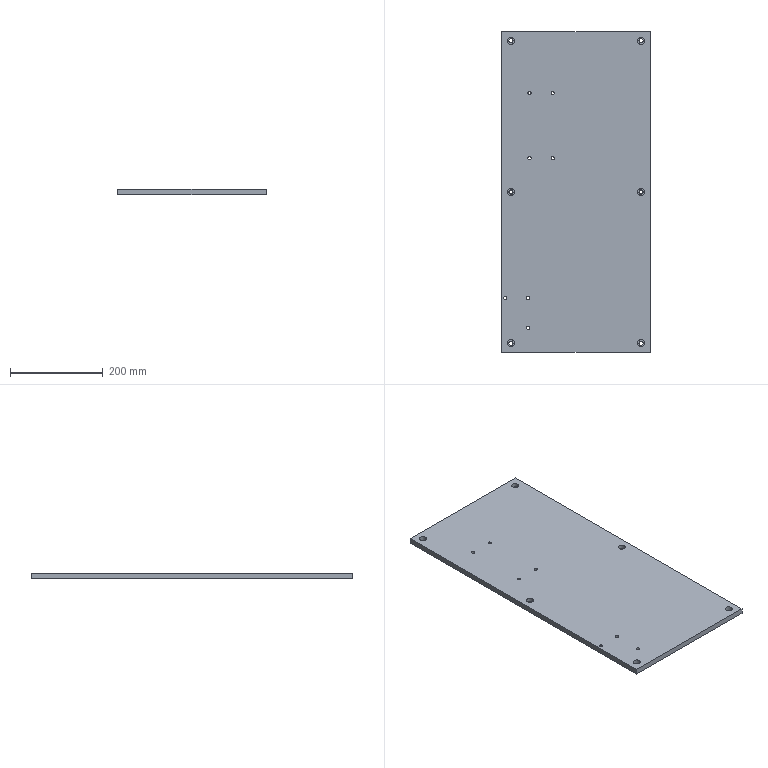Part | STEP file | X77-03005 | 1 solid | 50 faces | box 320 x 690 x 12 mm | volume 2635862 mm3 | cylinder 38 | plane 12 | commonest cylinder face diameters 6.8 x14 9 x12 15 x12
STEP:
#1=CARTESIAN_POINT('',(-213.4,557.5,0.));
#2=VERTEX_POINT('',#1);
#3=CARTESIAN_POINT('',(-206.6,557.5,0.));
#4=VERTEX_POINT('',#3);
#5=CARTESIAN_POINT('',(-210.,557.5,0.));
#6=DIRECTION('',(0.,0.,1.));
#7=DIRECTION('',(1.,0.,0.));
#8=AXIS2_PLACEMENT_3D('',#5,#6,#7);
#9=CIRCLE('',#8,3.4);
#10=EDGE_CURVE('',#2,#4,#9,.T.);
#11=ORIENTED_EDGE('',*,*,#10,.F.);
#12=CARTESIAN_POINT('',(-213.4,557.5,12.));
#13=VERTEX_POINT('',#12);
#14=CARTESIAN_POINT('',(-213.4,557.5,12.));
#15=DIRECTION('',(0.,0.,1.));
#16=VECTOR('',#15,1000.);
#17=LINE('',#14,#16);
#18=EDGE_CURVE('',#2,#13,#17,.T.);
#19=ORIENTED_EDGE('',*,*,#18,.T.);
#20=CARTESIAN_POINT('',(-206.6,557.5,12.));
#21=VERTEX_POINT('',#20);
#22=CARTESIAN_POINT('',(-210.,557.5,12.));
#23=DIRECTION('',(0.,0.,1.));
#24=DIRECTION('',(1.,0.,0.));
#25=AXIS2_PLACEMENT_3D('',#22,#23,#24);
#26=CIRCLE('',#25,3.4);
#27=EDGE_CURVE('',#13,#21,#26,.T.);
#28=ORIENTED_EDGE('',*,*,#27,.T.);
#29=CARTESIAN_POINT('',(-206.6,557.5,12.));
#30=DIRECTION('',(0.,0.,1.));
#31=VECTOR('',#30,1000.);
#32=LINE('',#29,#31);
#33=EDGE_CURVE('',#4,#21,#32,.T.);
#34=ORIENTED_EDGE('',*,*,#33,.F.);
#35=EDGE_LOOP('',(#11,#19,#28,#34));
#36=FACE_OUTER_BOUND('',#35,.T.);
#37=CARTESIAN_POINT('',(-210.,557.5,12.));
#38=DIRECTION('',(0.,0.,1.));
#39=DIRECTION('',(1.,0.,0.));
#40=AXIS2_PLACEMENT_3D('',#37,#38,#39);
#41=CYLINDRICAL_SURFACE('',#40,3.4);
#42=ADVANCED_FACE('',(#36),#41,.F.);
#43=CARTESIAN_POINT('',(-263.4,557.5,0.));
#44=VERTEX_POINT('',#43);
#45=CARTESIAN_POINT('',(-256.6,557.5,0.));
#46=VERTEX_POINT('',#45);
#47=CARTESIAN_POINT('',(-260.,557.5,0.));
#48=DIRECTION('',(0.,0.,1.));
#49=DIRECTION('',(1.,0.,0.));
#50=AXIS2_PLACEMENT_3D('',#47,#48,#49);
#51=CIRCLE('',#50,3.4);
#52=EDGE_CURVE('',#44,#46,#51,.T.);
#53=ORIENTED_EDGE('',*,*,#52,.F.);
#54=CARTESIAN_POINT('',(-263.4,557.5,12.));
#55=VERTEX_POINT('',#54);
#56=CARTESIAN_POINT('',(-263.4,557.5,12.));
#57=DIRECTION('',(0.,0.,1.));
#58=VECTOR('',#57,1000.);
#59=LINE('',#56,#58);
#60=EDGE_CURVE('',#44,#55,#59,.T.);
#61=ORIENTED_EDGE('',*,*,#60,.T.);
#62=CARTESIAN_POINT('',(-256.6,557.5,12.));
#63=VERTEX_POINT('',#62);
#64=CARTESIAN_POINT('',(-260.,557.5,12.));
#65=DIRECTION('',(0.,0.,1.));
#66=DIRECTION('',(1.,0.,0.));
#67=AXIS2_PLACEMENT_3D('',#64,#65,#66);
#68=CIRCLE('',#67,3.4);
#69=EDGE_CURVE('',#55,#63,#68,.T.);
#70=ORIENTED_EDGE('',*,*,#69,.T.);
#71=CARTESIAN_POINT('',(-256.6,557.5,12.));
#72=DIRECTION('',(0.,0.,1.));
#73=VECTOR('',#72,1000.);
#74=LINE('',#71,#73);
#75=EDGE_CURVE('',#46,#63,#74,.T.);
#76=ORIENTED_EDGE('',*,*,#75,.F.);
#77=EDGE_LOOP('',(#53,#61,#70,#76));
#78=FACE_OUTER_BOUND('',#77,.T.);
#79=CARTESIAN_POINT('',(-260.,557.5,12.));
#80=DIRECTION('',(0.,0.,1.));
#81=DIRECTION('',(1.,0.,0.));
#82=AXIS2_PLACEMENT_3D('',#79,#80,#81);
#83=CYLINDRICAL_SURFACE('',#82,3.4);
#84=ADVANCED_FACE('',(#78),#83,.F.);
#85=CARTESIAN_POINT('',(-213.4,417.5,0.));
#86=VERTEX_POINT('',#85);
#87=CARTESIAN_POINT('',(-206.6,417.5,0.));
#88=VERTEX_POINT('',#87);
#89=CARTESIAN_POINT('',(-210.,417.5,0.));
#90=DIRECTION('',(0.,0.,1.));
#91=DIRECTION('',(1.,0.,0.));
#92=AXIS2_PLACEMENT_3D('',#89,#90,#91);
#93=CIRCLE('',#92,3.4);
#94=EDGE_CURVE('',#86,#88,#93,.T.);
#95=ORIENTED_EDGE('',*,*,#94,.F.);
#96=CARTESIAN_POINT('',(-213.4,417.5,12.));
#97=VERTEX_POINT('',#96);
#98=CARTESIAN_POINT('',(-213.4,417.5,12.));
#99=DIRECTION('',(0.,0.,1.));
#100=VECTOR('',#99,1000.);
#101=LINE('',#98,#100);
#102=EDGE_CURVE('',#86,#97,#101,.T.);
#103=ORIENTED_EDGE('',*,*,#102,.T.);
#104=CARTESIAN_POINT('',(-206.6,417.5,12.));
#105=VERTEX_POINT('',#104);
#106=CARTESIAN_POINT('',(-210.,417.5,12.));
#107=DIRECTION('',(0.,0.,1.));
#108=DIRECTION('',(1.,0.,0.));
#109=AXIS2_PLACEMENT_3D('',#106,#107,#108);
#110=CIRCLE('',#109,3.4);
#111=EDGE_CURVE('',#97,#105,#110,.T.);
#112=ORIENTED_EDGE('',*,*,#111,.T.);
#113=CARTESIAN_POINT('',(-206.6,417.5,12.));
#114=DIRECTION('',(0.,0.,1.));
#115=VECTOR('',#114,1000.);
#116=LINE('',#113,#115);
#117=EDGE_CURVE('',#88,#105,#116,.T.);
#118=ORIENTED_EDGE('',*,*,#117,.F.);
#119=EDGE_LOOP('',(#95,#103,#112,#118));
#120=FACE_OUTER_BOUND('',#119,.T.);
#121=CARTESIAN_POINT('',(-210.,417.5,12.));
#122=DIRECTION('',(0.,0.,1.));
#123=DIRECTION('',(1.,0.,0.));
#124=AXIS2_PLACEMENT_3D('',#121,#122,#123);
#125=CYLINDRICAL_SURFACE('',#124,3.4);
#126=ADVANCED_FACE('',(#120),#125,.F.);
#127=CARTESIAN_POINT('',(-263.4,417.5,0.));
#128=VERTEX_POINT('',#127);
#129=CARTESIAN_POINT('',(-256.6,417.5,0.));
#130=VERTEX_POINT('',#129);
#131=CARTESIAN_POINT('',(-260.,417.5,0.));
#132=DIRECTION('',(0.,0.,1.));
#133=DIRECTION('',(1.,0.,0.));
#134=AXIS2_PLACEMENT_3D('',#131,#132,#133);
#135=CIRCLE('',#134,3.4);
#136=EDGE_CURVE('',#128,#130,#135,.T.);
#137=ORIENTED_EDGE('',*,*,#136,.F.);
#138=CARTESIAN_POINT('',(-263.4,417.5,12.));
#139=VERTEX_POINT('',#138);
#140=CARTESIAN_POINT('',(-263.4,417.5,12.));
#141=DIRECTION('',(0.,0.,1.));
#142=VECTOR('',#141,1000.);
#143=LINE('',#140,#142);
#144=EDGE_CURVE('',#128,#139,#143,.T.);
#145=ORIENTED_EDGE('',*,*,#144,.T.);
#146=CARTESIAN_POINT('',(-256.6,417.5,12.));
#147=VERTEX_POINT('',#146);
#148=CARTESIAN_POINT('',(-260.,417.5,12.));
#149=DIRECTION('',(0.,0.,1.));
#150=DIRECTION('',(1.,0.,0.));
#151=AXIS2_PLACEMENT_3D('',#148,#149,#150);
#152=CIRCLE('',#151,3.4);
#153=EDGE_CURVE('',#139,#147,#152,.T.);
#154=ORIENTED_EDGE('',*,*,#153,.T.);
#155=CARTESIAN_POINT('',(-256.6,417.5,12.));
#156=DIRECTION('',(0.,0.,1.));
#157=VECTOR('',#156,1000.);
#158=LINE('',#155,#157);
#159=EDGE_CURVE('',#130,#147,#158,.T.);
#160=ORIENTED_EDGE('',*,*,#159,.F.);
#161=EDGE_LOOP('',(#137,#145,#154,#160));
#162=FACE_OUTER_BOUND('',#161,.T.);
#163=CARTESIAN_POINT('',(-260.,417.5,12.));
#164=DIRECTION('',(0.,0.,1.));
#165=DIRECTION('',(1.,0.,0.));
#166=AXIS2_PLACEMENT_3D('',#163,#164,#165);
#167=CYLINDRICAL_SURFACE('',#166,3.4);
#168=ADVANCED_FACE('',(#162),#167,.F.);
#169=CARTESIAN_POINT('',(-266.4,117.,0.));
#170=VERTEX_POINT('',#169);
#171=CARTESIAN_POINT('',(-259.6,117.,0.));
#172=VERTEX_POINT('',#171);
#173=CARTESIAN_POINT('',(-263.,117.,0.));
#174=DIRECTION('',(0.,0.,1.));
#175=DIRECTION('',(1.,0.,0.));
#176=AXIS2_PLACEMENT_3D('',#173,#174,#175);
#177=CIRCLE('',#176,3.4);
#178=EDGE_CURVE('',#170,#172,#177,.T.);
#179=ORIENTED_EDGE('',*,*,#178,.F.);
#180=CARTESIAN_POINT('',(-266.4,117.,12.));
#181=VERTEX_POINT('',#180);
#182=CARTESIAN_POINT('',(-266.4,117.,12.));
#183=DIRECTION('',(0.,0.,1.));
#184=VECTOR('',#183,1000.);
#185=LINE('',#182,#184);
#186=EDGE_CURVE('',#170,#181,#185,.T.);
#187=ORIENTED_EDGE('',*,*,#186,.T.);
#188=CARTESIAN_POINT('',(-259.6,117.,12.));
#189=VERTEX_POINT('',#188);
#190=CARTESIAN_POINT('',(-263.,117.,12.));
#191=DIRECTION('',(0.,0.,1.));
#192=DIRECTION('',(1.,0.,0.));
#193=AXIS2_PLACEMENT_3D('',#190,#191,#192);
#194=CIRCLE('',#193,3.4);
#195=EDGE_CURVE('',#181,#189,#194,.T.);
#196=ORIENTED_EDGE('',*,*,#195,.T.);
#197=CARTESIAN_POINT('',(-259.6,117.,12.));
#198=DIRECTION('',(0.,0.,1.));
#199=VECTOR('',#198,1000.);
#200=LINE('',#197,#199);
#201=EDGE_CURVE('',#172,#189,#200,.T.);
#202=ORIENTED_EDGE('',*,*,#201,.F.);
#203=EDGE_LOOP('',(#179,#187,#196,#202));
#204=FACE_OUTER_BOUND('',#203,.T.);
#205=CARTESIAN_POINT('',(-263.,117.,12.));
#206=DIRECTION('',(0.,0.,1.));
#207=DIRECTION('',(1.,0.,0.));
#208=AXIS2_PLACEMENT_3D('',#205,#206,#207);
#209=CYLINDRICAL_SURFACE('',#208,3.4);
#210=ADVANCED_FACE('',(#204),#209,.F.);
#211=CARTESIAN_POINT('',(-266.4,53.,0.));
#212=VERTEX_POINT('',#211);
#213=CARTESIAN_POINT('',(-259.6,53.,0.));
#214=VERTEX_POINT('',#213);
#215=CARTESIAN_POINT('',(-263.,53.,0.));
#216=DIRECTION('',(0.,0.,1.));
#217=DIRECTION('',(1.,0.,0.));
#218=AXIS2_PLACEMENT_3D('',#215,#216,#217);
#219=CIRCLE('',#218,3.4);
#220=EDGE_CURVE('',#212,#214,#219,.T.);
#221=ORIENTED_EDGE('',*,*,#220,.F.);
#222=CARTESIAN_POINT('',(-266.4,53.,12.));
#223=VERTEX_POINT('',#222);
#224=CARTESIAN_POINT('',(-266.4,53.,12.));
#225=DIRECTION('',(0.,0.,1.));
#226=VECTOR('',#225,1000.);
#227=LINE('',#224,#226);
#228=EDGE_CURVE('',#212,#223,#227,.T.);
#229=ORIENTED_EDGE('',*,*,#228,.T.);
#230=CARTESIAN_POINT('',(-259.6,53.,12.));
#231=VERTEX_POINT('',#230);
#232=CARTESIAN_POINT('',(-263.,53.,12.));
#233=DIRECTION('',(0.,0.,1.));
#234=DIRECTION('',(1.,0.,0.));
#235=AXIS2_PLACEMENT_3D('',#232,#233,#234);
#236=CIRCLE('',#235,3.4);
#237=EDGE_CURVE('',#223,#231,#236,.T.);
#238=ORIENTED_EDGE('',*,*,#237,.T.);
#239=CARTESIAN_POINT('',(-259.6,53.,12.));
#240=DIRECTION('',(0.,0.,1.));
#241=VECTOR('',#240,1000.);
#242=LINE('',#239,#241);
#243=EDGE_CURVE('',#214,#231,#242,.T.);
#244=ORIENTED_EDGE('',*,*,#243,.F.);
#245=EDGE_LOOP('',(#221,#229,#238,#244));
#246=FACE_OUTER_BOUND('',#245,.T.);
#247=CARTESIAN_POINT('',(-263.,53.,12.));
#248=DIRECTION('',(0.,0.,1.));
#249=DIRECTION('',(1.,0.,0.));
#250=AXIS2_PLACEMENT_3D('',#247,#248,#249);
#251=CYLINDRICAL_SURFACE('',#250,3.4);
#252=ADVANCED_FACE('',(#246),#251,.F.);
#253=CARTESIAN_POINT('',(-315.4,117.,0.));
#254=VERTEX_POINT('',#253);
#255=CARTESIAN_POINT('',(-308.6,117.,0.));
#256=VERTEX_POINT('',#255);
#257=CARTESIAN_POINT('',(-312.,117.,0.));
#258=DIRECTION('',(0.,0.,1.));
#259=DIRECTION('',(1.,0.,0.));
#260=AXIS2_PLACEMENT_3D('',#257,#258,#259);
#261=CIRCLE('',#260,3.4);
#262=EDGE_CURVE('',#254,#256,#261,.T.);
#263=ORIENTED_EDGE('',*,*,#262,.F.);
#264=CARTESIAN_POINT('',(-315.4,117.,12.));
#265=VERTEX_POINT('',#264);
#266=CARTESIAN_POINT('',(-315.4,117.,12.));
#267=DIRECTION('',(0.,0.,1.));
#268=VECTOR('',#267,1000.);
#269=LINE('',#266,#268);
#270=EDGE_CURVE('',#254,#265,#269,.T.);
#271=ORIENTED_EDGE('',*,*,#270,.T.);
#272=CARTESIAN_POINT('',(-308.6,117.,12.));
#273=VERTEX_POINT('',#272);
#274=CARTESIAN_POINT('',(-312.,117.,12.));
#275=DIRECTION('',(0.,0.,1.));
#276=DIRECTION('',(1.,0.,0.));
#277=AXIS2_PLACEMENT_3D('',#274,#275,#276);
#278=CIRCLE('',#277,3.4);
#279=EDGE_CURVE('',#265,#273,#278,.T.);
#280=ORIENTED_EDGE('',*,*,#279,.T.);
#281=CARTESIAN_POINT('',(-308.6,117.,12.));
#282=DIRECTION('',(0.,0.,1.));
#283=VECTOR('',#282,1000.);
#284=LINE('',#281,#283);
#285=EDGE_CURVE('',#256,#273,#284,.T.);
#286=ORIENTED_EDGE('',*,*,#285,.F.);
#287=EDGE_LOOP('',(#263,#271,#280,#286));
#288=FACE_OUTER_BOUND('',#287,.T.);
#289=CARTESIAN_POINT('',(-312.,117.,12.));
#290=DIRECTION('',(0.,0.,1.));
#291=DIRECTION('',(1.,0.,0.));
#292=AXIS2_PLACEMENT_3D('',#289,#290,#291);
#293=CYLINDRICAL_SURFACE('',#292,3.4);
#294=ADVANCED_FACE('',(#288),#293,.F.);
#295=CARTESIAN_POINT('',(-27.5,670.,3.));
#296=VERTEX_POINT('',#295);
#297=CARTESIAN_POINT('',(-12.5,670.,3.));
#298=VERTEX_POINT('',#297);
#299=CARTESIAN_POINT('',(-20.,670.,3.));
#300=DIRECTION('',(0.,0.,1.));
#301=DIRECTION('',(1.,0.,0.));
#302=AXIS2_PLACEMENT_3D('',#299,#300,#301);
#303=CIRCLE('',#302,7.5);
#304=EDGE_CURVE('',#296,#298,#303,.T.);
#305=ORIENTED_EDGE('',*,*,#304,.F.);
#306=CARTESIAN_POINT('',(-27.5,670.,12.));
#307=VERTEX_POINT('',#306);
#308=CARTESIAN_POINT('',(-27.5,670.,12.));
#309=DIRECTION('',(0.,0.,1.));
#310=VECTOR('',#309,1000.);
#311=LINE('',#308,#310);
#312=EDGE_CURVE('',#296,#307,#311,.T.);
#313=ORIENTED_EDGE('',*,*,#312,.T.);
#314=CARTESIAN_POINT('',(-12.5,670.,12.));
#315=VERTEX_POINT('',#314);
#316=CARTESIAN_POINT('',(-20.,670.,12.));
#317=DIRECTION('',(0.,0.,1.));
#318=DIRECTION('',(1.,0.,0.));
#319=AXIS2_PLACEMENT_3D('',#316,#317,#318);
#320=CIRCLE('',#319,7.5);
#321=EDGE_CURVE('',#307,#315,#320,.T.);
#322=ORIENTED_EDGE('',*,*,#321,.T.);
#323=CARTESIAN_POINT('',(-12.5,670.,12.));
#324=DIRECTION('',(0.,0.,1.));
#325=VECTOR('',#324,1000.);
#326=LINE('',#323,#325);
#327=EDGE_CURVE('',#298,#315,#326,.T.);
#328=ORIENTED_EDGE('',*,*,#327,.F.);
#329=EDGE_LOOP('',(#305,#313,#322,#328));
#330=FACE_OUTER_BOUND('',#329,.T.);
#331=CARTESIAN_POINT('',(-20.,670.,12.));
#332=DIRECTION('',(0.,0.,1.));
#333=DIRECTION('',(1.,0.,0.));
#334=AXIS2_PLACEMENT_3D('',#331,#332,#333);
#335=CYLINDRICAL_SURFACE('',#334,7.5);
#336=ADVANCED_FACE('',(#330),#335,.F.);
#337=CARTESIAN_POINT('',(-24.5,670.,0.));
#338=VERTEX_POINT('',#337);
#339=CARTESIAN_POINT('',(-15.5,670.,0.));
#340=VERTEX_POINT('',#339);
#341=CARTESIAN_POINT('',(-20.,670.,0.));
#342=DIRECTION('',(0.,0.,1.));
#343=DIRECTION('',(1.,0.,0.));
#344=AXIS2_PLACEMENT_3D('',#341,#342,#343);
#345=CIRCLE('',#344,4.5);
#346=EDGE_CURVE('',#338,#340,#345,.T.);
#347=ORIENTED_EDGE('',*,*,#346,.F.);
#348=CARTESIAN_POINT('',(-24.5,670.,3.));
#349=VERTEX_POINT('',#348);
#350=CARTESIAN_POINT('',(-24.5,670.,12.));
#351=DIRECTION('',(0.,0.,1.));
#352=VECTOR('',#351,1000.);
#353=LINE('',#350,#352);
#354=EDGE_CURVE('',#338,#349,#353,.T.);
#355=ORIENTED_EDGE('',*,*,#354,.T.);
#356=CARTESIAN_POINT('',(-15.5,670.,3.));
#357=VERTEX_POINT('',#356);
#358=CARTESIAN_POINT('',(-20.,670.,3.));
#359=DIRECTION('',(0.,0.,1.));
#360=DIRECTION('',(1.,0.,0.));
#361=AXIS2_PLACEMENT_3D('',#358,#359,#360);
#362=CIRCLE('',#361,4.5);
#363=EDGE_CURVE('',#349,#357,#362,.T.);
#364=ORIENTED_EDGE('',*,*,#363,.T.);
#365=CARTESIAN_POINT('',(-15.5,670.,12.));
#366=DIRECTION('',(0.,0.,1.));
#367=VECTOR('',#366,1000.);
#368=LINE('',#365,#367);
#369=EDGE_CURVE('',#340,#357,#368,.T.);
#370=ORIENTED_EDGE('',*,*,#369,.F.);
#371=EDGE_LOOP('',(#347,#355,#364,#370));
#372=FACE_OUTER_BOUND('',#371,.T.);
#373=CARTESIAN_POINT('',(-20.,670.,12.));
#374=DIRECTION('',(0.,0.,1.));
#375=DIRECTION('',(1.,0.,0.));
#376=AXIS2_PLACEMENT_3D('',#373,#374,#375);
#377=CYLINDRICAL_SURFACE('',#376,4.5);
#378=ADVANCED_FACE('',(#372),#377,.F.);
#379=CARTESIAN_POINT('',(-307.5,20.,3.));
#380=VERTEX_POINT('',#379);
#381=CARTESIAN_POINT('',(-292.5,20.,3.));
#382=VERTEX_POINT('',#381);
#383=CARTESIAN_POINT('',(-300.,20.,3.));
#384=DIRECTION('',(0.,0.,1.));
#385=DIRECTION('',(1.,0.,0.));
#386=AXIS2_PLACEMENT_3D('',#383,#384,#385);
#387=CIRCLE('',#386,7.5);
#388=EDGE_CURVE('',#380,#382,#387,.T.);
#389=ORIENTED_EDGE('',*,*,#388,.F.);
#390=CARTESIAN_POINT('',(-307.5,20.,12.));
#391=VERTEX_POINT('',#390);
#392=CARTESIAN_POINT('',(-307.5,20.,12.));
#393=DIRECTION('',(0.,0.,1.));
#394=VECTOR('',#393,1000.);
#395=LINE('',#392,#394);
#396=EDGE_CURVE('',#380,#391,#395,.T.);
#397=ORIENTED_EDGE('',*,*,#396,.T.);
#398=CARTESIAN_POINT('',(-292.5,20.,12.));
#399=VERTEX_POINT('',#398);
#400=CARTESIAN_POINT('',(-300.,20.,12.));
#401=DIRECTION('',(0.,0.,1.));
#402=DIRECTION('',(1.,0.,0.));
#403=AXIS2_PLACEMENT_3D('',#400,#401,#402);
#404=CIRCLE('',#403,7.5);
#405=EDGE_CURVE('',#391,#399,#404,.T.);
#406=ORIENTED_EDGE('',*,*,#405,.T.);
#407=CARTESIAN_POINT('',(-292.5,20.,12.));
#408=DIRECTION('',(0.,0.,1.));
#409=VECTOR('',#408,1000.);
#410=LINE('',#407,#409);
#411=EDGE_CURVE('',#382,#399,#410,.T.);
#412=ORIENTED_EDGE('',*,*,#411,.F.);
#413=EDGE_LOOP('',(#389,#397,#406,#412));
#414=FACE_OUTER_BOUND('',#413,.T.);
#415=CARTESIAN_POINT('',(-300.,20.,12.));
#416=DIRECTION('',(0.,0.,1.));
#417=DIRECTION('',(1.,0.,0.));
#418=AXIS2_PLACEMENT_3D('',#415,#416,#417);
#419=CYLINDRICAL_SURFACE('',#418,7.5);
#420=ADVANCED_FACE('',(#414),#419,.F.);
#421=CARTESIAN_POINT('',(-304.5,20.,0.));
#422=VERTEX_POINT('',#421);
#423=CARTESIAN_POINT('',(-295.5,20.,0.));
#424=VERTEX_POINT('',#423);
#425=CARTESIAN_POINT('',(-300.,20.,0.));
#426=DIRECTION('',(0.,0.,1.));
#427=DIRECTION('',(1.,0.,0.));
#428=AXIS2_PLACEMENT_3D('',#425,#426,#427);
#429=CIRCLE('',#428,4.5);
#430=EDGE_CURVE('',#422,#424,#429,.T.);
#431=ORIENTED_EDGE('',*,*,#430,.F.);
#432=CARTESIAN_POINT('',(-304.5,20.,3.));
#433=VERTEX_POINT('',#432);
#434=CARTESIAN_POINT('',(-304.5,20.,12.));
#435=DIRECTION('',(0.,0.,1.));
#436=VECTOR('',#435,1000.);
#437=LINE('',#434,#436);
#438=EDGE_CURVE('',#422,#433,#437,.T.);
#439=ORIENTED_EDGE('',*,*,#438,.T.);
#440=CARTESIAN_POINT('',(-295.5,20.,3.));
#441=VERTEX_POINT('',#440);
#442=CARTESIAN_POINT('',(-300.,20.,3.));
#443=DIRECTION('',(0.,0.,1.));
#444=DIRECTION('',(1.,0.,0.));
#445=AXIS2_PLACEMENT_3D('',#442,#443,#444);
#446=CIRCLE('',#445,4.5);
#447=EDGE_CURVE('',#433,#441,#446,.T.);
#448=ORIENTED_EDGE('',*,*,#447,.T.);
#449=CARTESIAN_POINT('',(-295.5,20.,12.));
#450=DIRECTION('',(0.,0.,1.));
#451=VECTOR('',#450,1000.);
#452=LINE('',#449,#451);
#453=EDGE_CURVE('',#424,#441,#452,.T.);
#454=ORIENTED_EDGE('',*,*,#453,.F.);
#455=EDGE_LOOP('',(#431,#439,#448,#454));
#456=FACE_OUTER_BOUND('',#455,.T.);
#457=CARTESIAN_POINT('',(-300.,20.,12.));
#458=DIRECTION('',(0.,0.,1.));
#459=DIRECTION('',(1.,0.,0.));
#460=AXIS2_PLACEMENT_3D('',#457,#458,#459);
#461=CYLINDRICAL_SURFACE('',#460,4.5);
#462=ADVANCED_FACE('',(#456),#461,.F.);
#463=CARTESIAN_POINT('',(-27.5,345.,3.));
#464=VERTEX_POINT('',#463);
#465=CARTESIAN_POINT('',(-12.5,345.,3.));
#466=VERTEX_POINT('',#465);
#467=CARTESIAN_POINT('',(-20.,345.,3.));
#468=DIRECTION('',(0.,0.,1.));
#469=DIRECTION('',(1.,0.,0.));
#470=AXIS2_PLACEMENT_3D('',#467,#468,#469);
#471=CIRCLE('',#470,7.5);
#472=EDGE_CURVE('',#464,#466,#471,.T.);
#473=ORIENTED_EDGE('',*,*,#472,.F.);
#474=CARTESIAN_POINT('',(-27.5,345.,12.));
#475=VERTEX_POINT('',#474);
#476=CARTESIAN_POINT('',(-27.5,345.,12.));
#477=DIRECTION('',(0.,0.,1.));
#478=VECTOR('',#477,1000.);
#479=LINE('',#476,#478);
#480=EDGE_CURVE('',#464,#475,#479,.T.);
#481=ORIENTED_EDGE('',*,*,#480,.T.);
#482=CARTESIAN_POINT('',(-12.5,345.,12.));
#483=VERTEX_POINT('',#482);
#484=CARTESIAN_POINT('',(-20.,345.,12.));
#485=DIRECTION('',(0.,0.,1.));
#486=DIRECTION('',(1.,0.,0.));
#487=AXIS2_PLACEMENT_3D('',#484,#485,#486);
#488=CIRCLE('',#487,7.5);
#489=EDGE_CURVE('',#475,#483,#488,.T.);
#490=ORIENTED_EDGE('',*,*,#489,.T.);
#491=CARTESIAN_POINT('',(-12.5,345.,12.));
#492=DIRECTION('',(0.,0.,1.));
#493=VECTOR('',#492,1000.);
#494=LINE('',#491,#493);
#495=EDGE_CURVE('',#466,#483,#494,.T.);
#496=ORIENTED_EDGE('',*,*,#495,.F.);
#497=EDGE_LOOP('',(#473,#481,#490,#496));
#498=FACE_OUTER_BOUND('',#497,.T.);
#499=CARTESIAN_POINT('',(-20.,345.,12.));
#500=DIRECTION('',(0.,0.,1.));
#501=DIRECTION('',(1.,0.,0.));
#502=AXIS2_PLACEMENT_3D('',#499,#500,#501);
#503=CYLINDRICAL_SURFACE('',#502,7.5);
#504=ADVANCED_FACE('',(#498),#503,.F.);
#505=CARTESIAN_POINT('',(-24.5,345.,0.));
#506=VERTEX_POINT('',#505);
#507=CARTESIAN_POINT('',(-15.5,345.,0.));
#508=VERTEX_POINT('',#507);
#509=CARTESIAN_POINT('',(-20.,345.,0.));
#510=DIRECTION('',(0.,0.,1.));
#511=DIRECTION('',(1.,0.,0.));
#512=AXIS2_PLACEMENT_3D('',#509,#510,#511);
#513=CIRCLE('',#512,4.5);
#514=EDGE_CURVE('',#506,#508,#513,.T.);
#515=ORIENTED_EDGE('',*,*,#514,.F.);
#516=CARTESIAN_POINT('',(-24.5,345.,3.));
#517=VERTEX_POINT('',#516);
#518=CARTESIAN_POINT('',(-24.5,345.,12.));
#519=DIRECTION('',(0.,0.,1.));
#520=VECTOR('',#519,1000.);
#521=LINE('',#518,#520);
#522=EDGE_CURVE('',#506,#517,#521,.T.);
#523=ORIENTED_EDGE('',*,*,#522,.T.);
#524=CARTESIAN_POINT('',(-15.5,345.,3.));
#525=VERTEX_POINT('',#524);
#526=CARTESIAN_POINT('',(-20.,345.,3.));
#527=DIRECTION('',(0.,0.,1.));
#528=DIRECTION('',(1.,0.,0.));
#529=AXIS2_PLACEMENT_3D('',#526,#527,#528);
#530=CIRCLE('',#529,4.5);
#531=EDGE_CURVE('',#517,#525,#530,.T.);
#532=ORIENTED_EDGE('',*,*,#531,.T.);
#533=CARTESIAN_POINT('',(-15.5,345.,12.));
#534=DIRECTION('',(0.,0.,1.));
#535=VECTOR('',#534,1000.);
#536=LINE('',#533,#535);
#537=EDGE_CURVE('',#508,#525,#536,.T.);
#538=ORIENTED_EDGE('',*,*,#537,.F.);
#539=EDGE_LOOP('',(#515,#523,#532,#538));
#540=FACE_OUTER_BOUND('',#539,.T.);
#541=CARTESIAN_POINT('',(-20.,345.,12.));
#542=DIRECTION('',(0.,0.,1.));
#543=DIRECTION('',(1.,0.,0.));
#544=AXIS2_PLACEMENT_3D('',#541,#542,#543);
#545=CYLINDRICAL_SURFACE('',#544,4.5);
#546=ADVANCED_FACE('',(#540),#545,.F.);
#547=CARTESIAN_POINT('',(-27.5,20.,3.));
#548=VERTEX_POINT('',#547);
#549=CARTESIAN_POINT('',(-12.5,20.,3.));
#550=VERTEX_POINT('',#549);
#551=CARTESIAN_POINT('',(-20.,20.,3.));
#552=DIRECTION('',(0.,0.,1.));
#553=DIRECTION('',(1.,0.,0.));
#554=AXIS2_PLACEMENT_3D('',#551,#552,#553);
#555=CIRCLE('',#554,7.5);
#556=EDGE_CURVE('',#548,#550,#555,.T.);
#557=ORIENTED_EDGE('',*,*,#556,.F.);
#558=CARTESIAN_POINT('',(-27.5,20.,12.));
#559=VERTEX_POINT('',#558);
#560=CARTESIAN_POINT('',(-27.5,20.,12.));
#561=DIRECTION('',(0.,0.,1.));
#562=VECTOR('',#561,1000.);
#563=LINE('',#560,#562);
#564=EDGE_CURVE('',#548,#559,#563,.T.);
#565=ORIENTED_EDGE('',*,*,#564,.T.);
#566=CARTESIAN_POINT('',(-12.5,20.,12.));
#567=VERTEX_POINT('',#566);
#568=CARTESIAN_POINT('',(-20.,20.,12.));
#569=DIRECTION('',(0.,0.,1.));
#570=DIRECTION('',(1.,0.,0.));
#571=AXIS2_PLACEMENT_3D('',#568,#569,#570);
#572=CIRCLE('',#571,7.5);
#573=EDGE_CURVE('',#559,#567,#572,.T.);
#574=ORIENTED_EDGE('',*,*,#573,.T.);
#575=CARTESIAN_POINT('',(-12.5,20.,12.));
#576=DIRECTION('',(0.,0.,1.));
#577=VECTOR('',#576,1000.);
#578=LINE('',#575,#577);
#579=EDGE_CURVE('',#550,#567,#578,.T.);
#580=ORIENTED_EDGE('',*,*,#579,.F.);
#581=EDGE_LOOP('',(#557,#565,#574,#580));
#582=FACE_OUTER_BOUND('',#581,.T.);
#583=CARTESIAN_POINT('',(-20.,20.,12.));
#584=DIRECTION('',(0.,0.,1.));
#585=DIRECTION('',(1.,0.,0.));
#586=AXIS2_PLACEMENT_3D('',#583,#584,#585);
#587=CYLINDRICAL_SURFACE('',#586,7.5);
#588=ADVANCED_FACE('',(#582),#587,.F.);
#589=CARTESIAN_POINT('',(-24.5,20.,0.));
#590=VERTEX_POINT('',#589);
#591=CARTESIAN_POINT('',(-15.5,20.,0.));
#592=VERTEX_POINT('',#591);
#593=CARTESIAN_POINT('',(-20.,20.,0.));
#594=DIRECTION('',(0.,0.,1.));
#595=DIRECTION('',(1.,0.,0.));
#596=AXIS2_PLACEMENT_3D('',#593,#594,#595);
#597=CIRCLE('',#596,4.5);
#598=EDGE_CURVE('',#590,#592,#597,.T.);
#599=ORIENTED_EDGE('',*,*,#598,.F.);
#600=CARTESIAN_POINT('',(-24.5,20.,3.));
#601=VERTEX_POINT('',#600);
#602=CARTESIAN_POINT('',(-24.5,20.,12.));
#603=DIRECTION('',(0.,0.,1.));
#604=VECTOR('',#603,1000.);
#605=LINE('',#602,#604);
#606=EDGE_CURVE('',#590,#601,#605,.T.);
#607=ORIENTED_EDGE('',*,*,#606,.T.);
#608=CARTESIAN_POINT('',(-15.5,20.,3.));
#609=VERTEX_POINT('',#608);
#610=CARTESIAN_POINT('',(-20.,20.,3.));
#611=DIRECTION('',(0.,0.,1.));
#612=DIRECTION('',(1.,0.,0.));
#613=AXIS2_PLACEMENT_3D('',#610,#611,#612);
#614=CIRCLE('',#613,4.5);
#615=EDGE_CURVE('',#601,#609,#614,.T.);
#616=ORIENTED_EDGE('',*,*,#615,.T.);
#617=CARTESIAN_POINT('',(-15.5,20.,12.));
#618=DIRECTION('',(0.,0.,1.));
#619=VECTOR('',#618,1000.);
#620=LINE('',#617,#619);
#621=EDGE_CURVE('',#592,#609,#620,.T.);
#622=ORIENTED_EDGE('',*,*,#621,.F.);
#623=EDGE_LOOP('',(#599,#607,#616,#622));
#624=FACE_OUTER_BOUND('',#623,.T.);
#625=CARTESIAN_POINT('',(-20.,20.,12.));
#626=DIRECTION('',(0.,0.,1.));
#627=DIRECTION('',(1.,0.,0.));
#628=AXIS2_PLACEMENT_3D('',#625,#626,#627);
#629=CYLINDRICAL_SURFACE('',#628,4.5);
#630=ADVANCED_FACE('',(#624),#629,.F.);
#631=CARTESIAN_POINT('',(-307.5,345.,3.));
#632=VERTEX_POINT('',#631);
#633=CARTESIAN_POINT('',(-292.5,345.,3.));
#634=VERTEX_POINT('',#633);
#635=CARTESIAN_POINT('',(-300.,345.,3.));
#636=DIRECTION('',(0.,0.,1.));
#637=DIRECTION('',(1.,0.,0.));
#638=AXIS2_PLACEMENT_3D('',#635,#636,#637);
#639=CIRCLE('',#638,7.5);
#640=EDGE_CURVE('',#632,#634,#639,.T.);
#641=ORIENTED_EDGE('',*,*,#640,.F.);
#642=CARTESIAN_POINT('',(-307.5,345.,12.));
#643=VERTEX_POINT('',#642);
#644=CARTESIAN_POINT('',(-307.5,345.,12.));
#645=DIRECTION('',(0.,0.,1.));
#646=VECTOR('',#645,1000.);
#647=LINE('',#644,#646);
#648=EDGE_CURVE('',#632,#643,#647,.T.);
#649=ORIENTED_EDGE('',*,*,#648,.T.);
#650=CARTESIAN_POINT('',(-292.5,345.,12.));
#651=VERTEX_POINT('',#650);
#652=CARTESIAN_POINT('',(-300.,345.,12.));
#653=DIRECTION('',(0.,0.,1.));
#654=DIRECTION('',(1.,0.,0.));
#655=AXIS2_PLACEMENT_3D('',#652,#653,#654);
#656=CIRCLE('',#655,7.5);
#657=EDGE_CURVE('',#643,#651,#656,.T.);
#658=ORIENTED_EDGE('',*,*,#657,.T.);
#659=CARTESIAN_POINT('',(-292.5,345.,12.));
#660=DIRECTION('',(0.,0.,1.));
#661=VECTOR('',#660,1000.);
#662=LINE('',#659,#661);
#663=EDGE_CURVE('',#634,#651,#662,.T.);
#664=ORIENTED_EDGE('',*,*,#663,.F.);
#665=EDGE_LOOP('',(#641,#649,#658,#664));
#666=FACE_OUTER_BOUND('',#665,.T.);
#667=CARTESIAN_POINT('',(-300.,345.,12.));
#668=DIRECTION('',(0.,0.,1.));
#669=DIRECTION('',(1.,0.,0.));
#670=AXIS2_PLACEMENT_3D('',#667,#668,#669);
#671=CYLINDRICAL_SURFACE('',#670,7.5);
#672=ADVANCED_FACE('',(#666),#671,.F.);
#673=CARTESIAN_POINT('',(-304.5,345.,0.));
#674=VERTEX_POINT('',#673);
#675=CARTESIAN_POINT('',(-295.5,345.,0.));
#676=VERTEX_POINT('',#675);
#677=CARTESIAN_POINT('',(-300.,345.,0.));
#678=DIRECTION('',(0.,0.,1.));
#679=DIRECTION('',(1.,0.,0.));
#680=AXIS2_PLACEMENT_3D('',#677,#678,#679);
#681=CIRCLE('',#680,4.5);
#682=EDGE_CURVE('',#674,#676,#681,.T.);
#683=ORIENTED_EDGE('',*,*,#682,.F.);
#684=CARTESIAN_POINT('',(-304.5,345.,3.));
#685=VERTEX_POINT('',#684);
#686=CARTESIAN_POINT('',(-304.5,345.,12.));
#687=DIRECTION('',(0.,0.,1.));
#688=VECTOR('',#687,1000.);
#689=LINE('',#686,#688);
#690=EDGE_CURVE('',#674,#685,#689,.T.);
#691=ORIENTED_EDGE('',*,*,#690,.T.);
#692=CARTESIAN_POINT('',(-295.5,345.,3.));
#693=VERTEX_POINT('',#692);
#694=CARTESIAN_POINT('',(-300.,345.,3.));
#695=DIRECTION('',(0.,0.,1.));
#696=DIRECTION('',(1.,0.,0.));
#697=AXIS2_PLACEMENT_3D('',#694,#695,#696);
#698=CIRCLE('',#697,4.5);
#699=EDGE_CURVE('',#685,#693,#698,.T.);
#700=ORIENTED_EDGE('',*,*,#699,.T.);
#701=CARTESIAN_POINT('',(-295.5,345.,12.));
#702=DIRECTION('',(0.,0.,1.));
#703=VECTOR('',#702,1000.);
#704=LINE('',#701,#703);
#705=EDGE_CURVE('',#676,#693,#704,.T.);
#706=ORIENTED_EDGE('',*,*,#705,.F.);
#707=EDGE_LOOP('',(#683,#691,#700,#706));
#708=FACE_OUTER_BOUND('',#707,.T.);
#709=CARTESIAN_POINT('',(-300.,345.,12.));
#710=DIRECTION('',(0.,0.,1.));
#711=DIRECTION('',(1.,0.,0.));
#712=AXIS2_PLACEMENT_3D('',#709,#710,#711);
#713=CYLINDRICAL_SURFACE('',#712,4.5);
#714=ADVANCED_FACE('',(#708),#713,.F.);
#715=CARTESIAN_POINT('',(-307.5,670.,3.));
#716=VERTEX_POINT('',#715);
#717=CARTESIAN_POINT('',(-292.5,670.,3.));
#718=VERTEX_POINT('',#717);
#719=CARTESIAN_POINT('',(-300.,670.,3.));
#720=DIRECTION('',(0.,0.,1.));
#721=DIRECTION('',(1.,0.,0.));
#722=AXIS2_PLACEMENT_3D('',#719,#720,#721);
#723=CIRCLE('',#722,7.5);
#724=EDGE_CURVE('',#716,#718,#723,.T.);
#725=ORIENTED_EDGE('',*,*,#724,.F.);
#726=CARTESIAN_POINT('',(-307.5,670.,12.));
#727=VERTEX_POINT('',#726);
#728=CARTESIAN_POINT('',(-307.5,670.,12.));
#729=DIRECTION('',(0.,0.,1.));
#730=VECTOR('',#729,1000.);
#731=LINE('',#728,#730);
#732=EDGE_CURVE('',#716,#727,#731,.T.);
#733=ORIENTED_EDGE('',*,*,#732,.T.);
#734=CARTESIAN_POINT('',(-292.5,670.,12.));
#735=VERTEX_POINT('',#734);
#736=CARTESIAN_POINT('',(-300.,670.,12.));
#737=DIRECTION('',(0.,0.,1.));
#738=DIRECTION('',(1.,0.,0.));
#739=AXIS2_PLACEMENT_3D('',#736,#737,#738);
#740=CIRCLE('',#739,7.5);
#741=EDGE_CURVE('',#727,#735,#740,.T.);
#742=ORIENTED_EDGE('',*,*,#741,.T.);
#743=CARTESIAN_POINT('',(-292.5,670.,12.));
#744=DIRECTION('',(0.,0.,1.));
#745=VECTOR('',#744,1000.);
#746=LINE('',#743,#745);
#747=EDGE_CURVE('',#718,#735,#746,.T.);
#748=ORIENTED_EDGE('',*,*,#747,.F.);
#749=EDGE_LOOP('',(#725,#733,#742,#748));
#750=FACE_OUTER_BOUND('',#749,.T.);
#751=CARTESIAN_POINT('',(-300.,670.,12.));
#752=DIRECTION('',(0.,0.,1.));
#753=DIRECTION('',(1.,0.,0.));
#754=AXIS2_PLACEMENT_3D('',#751,#752,#753);
#755=CYLINDRICAL_SURFACE('',#754,7.5);
#756=ADVANCED_FACE('',(#750),#755,.F.);
#757=CARTESIAN_POINT('',(-304.5,670.,0.));
#758=VERTEX_POINT('',#757);
#759=CARTESIAN_POINT('',(-295.5,670.,0.));
#760=VERTEX_POINT('',#759);
#761=CARTESIAN_POINT('',(-300.,670.,0.));
#762=DIRECTION('',(0.,0.,1.));
#763=DIRECTION('',(1.,0.,0.));
#764=AXIS2_PLACEMENT_3D('',#761,#762,#763);
#765=CIRCLE('',#764,4.5);
#766=EDGE_CURVE('',#758,#760,#765,.T.);
#767=ORIENTED_EDGE('',*,*,#766,.F.);
#768=CARTESIAN_POINT('',(-304.5,670.,3.));
#769=VERTEX_POINT('',#768);
#770=CARTESIAN_POINT('',(-304.5,670.,12.));
#771=DIRECTION('',(0.,0.,1.));
#772=VECTOR('',#771,1000.);
#773=LINE('',#770,#772);
#774=EDGE_CURVE('',#758,#769,#773,.T.);
#775=ORIENTED_EDGE('',*,*,#774,.T.);
#776=CARTESIAN_POINT('',(-295.5,670.,3.));
#777=VERTEX_POINT('',#776);
#778=CARTESIAN_POINT('',(-300.,670.,3.));
#779=DIRECTION('',(0.,0.,1.));
#780=DIRECTION('',(1.,0.,0.));
#781=AXIS2_PLACEMENT_3D('',#778,#779,#780);
#782=CIRCLE('',#781,4.5);
#783=EDGE_CURVE('',#769,#777,#782,.T.);
#784=ORIENTED_EDGE('',*,*,#783,.T.);
#785=CARTESIAN_POINT('',(-295.5,670.,12.));
#786=DIRECTION('',(0.,0.,1.));
#787=VECTOR('',#786,1000.);
#788=LINE('',#785,#787);
#789=EDGE_CURVE('',#760,#777,#788,.T.);
#790=ORIENTED_EDGE('',*,*,#789,.F.);
#791=EDGE_LOOP('',(#767,#775,#784,#790));
#792=FACE_OUTER_BOUND('',#791,.T.);
#793=CARTESIAN_POINT('',(-300.,670.,12.));
#794=DIRECTION('',(0.,0.,1.));
#795=DIRECTION('',(1.,0.,0.));
#796=AXIS2_PLACEMENT_3D('',#793,#794,#795);
#797=CYLINDRICAL_SURFACE('',#796,4.5);
#798=ADVANCED_FACE('',(#792),#797,.F.);
#799=CARTESIAN_POINT('',(0.,0.,0.));
#800=VERTEX_POINT('',#799);
#801=CARTESIAN_POINT('',(0.,690.,0.));
#802=VERTEX_POINT('',#801);
#803=CARTESIAN_POINT('',(0.,0.,0.));
#804=DIRECTION('',(0.,1.,0.));
#805=VECTOR('',#804,1000.);
#806=LINE('',#803,#805);
#807=EDGE_CURVE('',#800,#802,#806,.T.);
#808=ORIENTED_EDGE('',*,*,#807,.T.);
#809=CARTESIAN_POINT('',(0.,690.,12.));
#810=VERTEX_POINT('',#809);
#811=CARTESIAN_POINT('',(0.,690.,12.));
#812=DIRECTION('',(0.,0.,-1.));
#813=VECTOR('',#812,1000.);
#814=LINE('',#811,#813);
#815=EDGE_CURVE('',#810,#802,#814,.T.);
#816=ORIENTED_EDGE('',*,*,#815,.F.);
#817=CARTESIAN_POINT('',(0.,0.,12.));
#818=VERTEX_POINT('',#817);
#819=CARTESIAN_POINT('',(0.,0.,12.));
#820=DIRECTION('',(0.,1.,0.));
#821=VECTOR('',#820,1000.);
#822=LINE('',#819,#821);
#823=EDGE_CURVE('',#818,#810,#822,.T.);
#824=ORIENTED_EDGE('',*,*,#823,.F.);
#825=CARTESIAN_POINT('',(0.,0.,12.));
#826=DIRECTION('',(0.,0.,-1.));
#827=VECTOR('',#826,1000.);
#828=LINE('',#825,#827);
#829=EDGE_CURVE('',#818,#800,#828,.T.);
#830=ORIENTED_EDGE('',*,*,#829,.T.);
#831=EDGE_LOOP('',(#808,#816,#824,#830));
#832=FACE_OUTER_BOUND('',#831,.T.);
#833=CARTESIAN_POINT('',(0.,0.,12.));
#834=DIRECTION('',(-1.,0.,0.));
#835=DIRECTION('',(0.,0.,1.));
#836=AXIS2_PLACEMENT_3D('',#833,#834,#835);
#837=PLANE('',#836);
#838=ADVANCED_FACE('',(#832),#837,.F.);
#839=CARTESIAN_POINT('',(-320.,690.,0.));
#840=VERTEX_POINT('',#839);
#841=CARTESIAN_POINT('',(0.,690.,0.));
#842=DIRECTION('',(-1.,0.,0.));
#843=VECTOR('',#842,1000.);
#844=LINE('',#841,#843);
#845=EDGE_CURVE('',#802,#840,#844,.T.);
#846=ORIENTED_EDGE('',*,*,#845,.T.);
#847=CARTESIAN_POINT('',(-320.,690.,12.));
#848=VERTEX_POINT('',#847);
#849=CARTESIAN_POINT('',(-320.,690.,12.));
#850=DIRECTION('',(0.,0.,-1.));
#851=VECTOR('',#850,1000.);
#852=LINE('',#849,#851);
#853=EDGE_CURVE('',#848,#840,#852,.T.);
#854=ORIENTED_EDGE('',*,*,#853,.F.);
#855=CARTESIAN_POINT('',(0.,690.,12.));
#856=DIRECTION('',(-1.,0.,0.));
#857=VECTOR('',#856,1000.);
#858=LINE('',#855,#857);
#859=EDGE_CURVE('',#810,#848,#858,.T.);
#860=ORIENTED_EDGE('',*,*,#859,.F.);
#861=ORIENTED_EDGE('',*,*,#815,.T.);
#862=EDGE_LOOP('',(#846,#854,#860,#861));
#863=FACE_OUTER_BOUND('',#862,.T.);
#864=CARTESIAN_POINT('',(0.,690.,12.));
#865=DIRECTION('',(0.,-1.,0.));
#866=DIRECTION('',(0.,0.,-1.));
#867=AXIS2_PLACEMENT_3D('',#864,#865,#866);
#868=PLANE('',#867);
#869=ADVANCED_FACE('',(#863),#868,.F.);
#870=CARTESIAN_POINT('',(-320.,0.,0.));
#871=VERTEX_POINT('',#870);
#872=CARTESIAN_POINT('',(-320.,0.,0.));
#873=DIRECTION('',(0.,-1.,0.));
#874=VECTOR('',#873,1000.);
#875=LINE('',#872,#874);
#876=EDGE_CURVE('',#840,#871,#875,.T.);
#877=ORIENTED_EDGE('',*,*,#876,.T.);
#878=CARTESIAN_POINT('',(-320.,0.,12.));
#879=VERTEX_POINT('',#878);
#880=CARTESIAN_POINT('',(-320.,0.,12.));
#881=DIRECTION('',(0.,0.,-1.));
#882=VECTOR('',#881,1000.);
#883=LINE('',#880,#882);
#884=EDGE_CURVE('',#879,#871,#883,.T.);
#885=ORIENTED_EDGE('',*,*,#884,.F.);
#886=CARTESIAN_POINT('',(-320.,0.,12.));
#887=DIRECTION('',(0.,-1.,0.));
#888=VECTOR('',#887,1000.);
#889=LINE('',#886,#888);
#890=EDGE_CURVE('',#848,#879,#889,.T.);
#891=ORIENTED_EDGE('',*,*,#890,.F.);
#892=ORIENTED_EDGE('',*,*,#853,.T.);
#893=EDGE_LOOP('',(#877,#885,#891,#892));
#894=FACE_OUTER_BOUND('',#893,.T.);
#895=CARTESIAN_POINT('',(-320.,0.,12.));
#896=DIRECTION('',(1.,0.,0.));
#897=DIRECTION('',(0.,0.,-1.));
#898=AXIS2_PLACEMENT_3D('',#895,#896,#897);
#899=PLANE('',#898);
#900=ADVANCED_FACE('',(#894),#899,.F.);
#901=CARTESIAN_POINT('',(0.,0.,0.));
#902=DIRECTION('',(1.,0.,0.));
#903=VECTOR('',#902,1000.);
#904=LINE('',#901,#903);
#905=EDGE_CURVE('',#871,#800,#904,.T.);
#906=ORIENTED_EDGE('',*,*,#905,.T.);
#907=ORIENTED_EDGE('',*,*,#829,.F.);
#908=CARTESIAN_POINT('',(0.,0.,12.));
#909=DIRECTION('',(1.,0.,0.));
#910=VECTOR('',#909,1000.);
#911=LINE('',#908,#910);
#912=EDGE_CURVE('',#879,#818,#911,.T.);
#913=ORIENTED_EDGE('',*,*,#912,.F.);
#914=ORIENTED_EDGE('',*,*,#884,.T.);
#915=EDGE_LOOP('',(#906,#907,#913,#914));
#916=FACE_OUTER_BOUND('',#915,.T.);
#917=CARTESIAN_POINT('',(0.,0.,12.));
#918=DIRECTION('',(0.,1.,0.));
#919=DIRECTION('',(-1.,0.,0.));
#920=AXIS2_PLACEMENT_3D('',#917,#918,#919);
#921=PLANE('',#920);
#922=ADVANCED_FACE('',(#916),#921,.F.);
#923=CARTESIAN_POINT('',(-210.,557.5,12.));
#924=DIRECTION('',(0.,0.,1.));
#925=DIRECTION('',(1.,0.,0.));
#926=AXIS2_PLACEMENT_3D('',#923,#924,#925);
#927=CIRCLE('',#926,3.4);
#928=EDGE_CURVE('',#21,#13,#927,.T.);
#929=ORIENTED_EDGE('',*,*,#928,.F.);
#930=ORIENTED_EDGE('',*,*,#27,.F.);
#931=EDGE_LOOP('',(#929,#930));
#932=FACE_BOUND('',#931,.T.);
#933=CARTESIAN_POINT('',(-260.,557.5,12.));
#934=DIRECTION('',(0.,0.,1.));
#935=DIRECTION('',(1.,0.,0.));
#936=AXIS2_PLACEMENT_3D('',#933,#934,#935);
#937=CIRCLE('',#936,3.4);
#938=EDGE_CURVE('',#63,#55,#937,.T.);
#939=ORIENTED_EDGE('',*,*,#938,.F.);
#940=ORIENTED_EDGE('',*,*,#69,.F.);
#941=EDGE_LOOP('',(#939,#940));
#942=FACE_BOUND('',#941,.T.);
#943=CARTESIAN_POINT('',(-210.,417.5,12.));
#944=DIRECTION('',(0.,0.,1.));
#945=DIRECTION('',(1.,0.,0.));
#946=AXIS2_PLACEMENT_3D('',#943,#944,#945);
#947=CIRCLE('',#946,3.4);
#948=EDGE_CURVE('',#105,#97,#947,.T.);
#949=ORIENTED_EDGE('',*,*,#948,.F.);
#950=ORIENTED_EDGE('',*,*,#111,.F.);
#951=EDGE_LOOP('',(#949,#950));
#952=FACE_BOUND('',#951,.T.);
#953=CARTESIAN_POINT('',(-260.,417.5,12.));
#954=DIRECTION('',(0.,0.,1.));
#955=DIRECTION('',(1.,0.,0.));
#956=AXIS2_PLACEMENT_3D('',#953,#954,#955);
#957=CIRCLE('',#956,3.4);
#958=EDGE_CURVE('',#147,#139,#957,.T.);
#959=ORIENTED_EDGE('',*,*,#958,.F.);
#960=ORIENTED_EDGE('',*,*,#153,.F.);
#961=EDGE_LOOP('',(#959,#960));
#962=FACE_BOUND('',#961,.T.);
#963=CARTESIAN_POINT('',(-263.,117.,12.));
#964=DIRECTION('',(0.,0.,1.));
#965=DIRECTION('',(1.,0.,0.));
#966=AXIS2_PLACEMENT_3D('',#963,#964,#965);
#967=CIRCLE('',#966,3.4);
#968=EDGE_CURVE('',#189,#181,#967,.T.);
#969=ORIENTED_EDGE('',*,*,#968,.F.);
#970=ORIENTED_EDGE('',*,*,#195,.F.);
#971=EDGE_LOOP('',(#969,#970));
#972=FACE_BOUND('',#971,.T.);
#973=CARTESIAN_POINT('',(-263.,53.,12.));
#974=DIRECTION('',(0.,0.,1.));
#975=DIRECTION('',(1.,0.,0.));
#976=AXIS2_PLACEMENT_3D('',#973,#974,#975);
#977=CIRCLE('',#976,3.4);
#978=EDGE_CURVE('',#231,#223,#977,.T.);
#979=ORIENTED_EDGE('',*,*,#978,.F.);
#980=ORIENTED_EDGE('',*,*,#237,.F.);
#981=EDGE_LOOP('',(#979,#980));
#982=FACE_BOUND('',#981,.T.);
#983=CARTESIAN_POINT('',(-312.,117.,12.));
#984=DIRECTION('',(0.,0.,1.));
#985=DIRECTION('',(1.,0.,0.));
#986=AXIS2_PLACEMENT_3D('',#983,#984,#985);
#987=CIRCLE('',#986,3.4);
#988=EDGE_CURVE('',#273,#265,#987,.T.);
#989=ORIENTED_EDGE('',*,*,#988,.F.);
#990=ORIENTED_EDGE('',*,*,#279,.F.);
#991=EDGE_LOOP('',(#989,#990));
#992=FACE_BOUND('',#991,.T.);
#993=CARTESIAN_POINT('',(-20.,670.,12.));
#994=DIRECTION('',(0.,0.,1.));
#995=DIRECTION('',(1.,0.,0.));
#996=AXIS2_PLACEMENT_3D('',#993,#994,#995);
#997=CIRCLE('',#996,7.5);
#998=EDGE_CURVE('',#315,#307,#997,.T.);
#999=ORIENTED_EDGE('',*,*,#998,.F.);
#1000=ORIENTED_EDGE('',*,*,#321,.F.);
#1001=EDGE_LOOP('',(#999,#1000));
#1002=FACE_BOUND('',#1001,.T.);
#1003=CARTESIAN_POINT('',(-300.,20.,12.));
#1004=DIRECTION('',(0.,0.,1.));
#1005=DIRECTION('',(1.,0.,0.));
#1006=AXIS2_PLACEMENT_3D('',#1003,#1004,#1005);
#1007=CIRCLE('',#1006,7.5);
#1008=EDGE_CURVE('',#399,#391,#1007,.T.);
#1009=ORIENTED_EDGE('',*,*,#1008,.F.);
#1010=ORIENTED_EDGE('',*,*,#405,.F.);
#1011=EDGE_LOOP('',(#1009,#1010));
#1012=FACE_BOUND('',#1011,.T.);
#1013=CARTESIAN_POINT('',(-20.,345.,12.));
#1014=DIRECTION('',(0.,0.,1.));
#1015=DIRECTION('',(1.,0.,0.));
#1016=AXIS2_PLACEMENT_3D('',#1013,#1014,#1015);
#1017=CIRCLE('',#1016,7.5);
#1018=EDGE_CURVE('',#483,#475,#1017,.T.);
#1019=ORIENTED_EDGE('',*,*,#1018,.F.);
#1020=ORIENTED_EDGE('',*,*,#489,.F.);
#1021=EDGE_LOOP('',(#1019,#1020));
#1022=FACE_BOUND('',#1021,.T.);
#1023=CARTESIAN_POINT('',(-20.,20.,12.));
#1024=DIRECTION('',(0.,0.,1.));
#1025=DIRECTION('',(1.,0.,0.));
#1026=AXIS2_PLACEMENT_3D('',#1023,#1024,#1025);
#1027=CIRCLE('',#1026,7.5);
#1028=EDGE_CURVE('',#567,#559,#1027,.T.);
#1029=ORIENTED_EDGE('',*,*,#1028,.F.);
#1030=ORIENTED_EDGE('',*,*,#573,.F.);
#1031=EDGE_LOOP('',(#1029,#1030));
#1032=FACE_BOUND('',#1031,.T.);
#1033=CARTESIAN_POINT('',(-300.,345.,12.));
#1034=DIRECTION('',(0.,0.,1.));
#1035=DIRECTION('',(1.,0.,0.));
#1036=AXIS2_PLACEMENT_3D('',#1033,#1034,#1035);
#1037=CIRCLE('',#1036,7.5);
#1038=EDGE_CURVE('',#651,#643,#1037,.T.);
#1039=ORIENTED_EDGE('',*,*,#1038,.F.);
#1040=ORIENTED_EDGE('',*,*,#657,.F.);
#1041=EDGE_LOOP('',(#1039,#1040));
#1042=FACE_BOUND('',#1041,.T.);
#1043=CARTESIAN_POINT('',(-300.,670.,12.));
#1044=DIRECTION('',(0.,0.,1.));
#1045=DIRECTION('',(1.,0.,0.));
#1046=AXIS2_PLACEMENT_3D('',#1043,#1044,#1045);
#1047=CIRCLE('',#1046,7.5);
#1048=EDGE_CURVE('',#735,#727,#1047,.T.);
#1049=ORIENTED_EDGE('',*,*,#1048,.F.);
#1050=ORIENTED_EDGE('',*,*,#741,.F.);
#1051=EDGE_LOOP('',(#1049,#1050));
#1052=FACE_BOUND('',#1051,.T.);
#1053=ORIENTED_EDGE('',*,*,#823,.T.);
#1054=ORIENTED_EDGE('',*,*,#859,.T.);
#1055=ORIENTED_EDGE('',*,*,#890,.T.);
#1056=ORIENTED_EDGE('',*,*,#912,.T.);
#1057=EDGE_LOOP('',(#1053,#1054,#1055,#1056));
#1058=FACE_OUTER_BOUND('',#1057,.T.);
#1059=CARTESIAN_POINT('',(0.,690.,12.));
#1060=DIRECTION('',(0.,0.,1.));
#1061=DIRECTION('',(1.,0.,0.));
#1062=AXIS2_PLACEMENT_3D('',#1059,#1060,#1061);
#1063=PLANE('',#1062);
#1064=ADVANCED_FACE('',(#932,#942,#952,#962,#972,#982,#992,#1002,#1012,#1022,#1032,#1042,#1052,#1058),#1063,.T.);
#1065=CARTESIAN_POINT('',(-210.,557.5,0.));
#1066=DIRECTION('',(0.,0.,1.));
#1067=DIRECTION('',(1.,0.,0.));
#1068=AXIS2_PLACEMENT_3D('',#1065,#1066,#1067);
#1069=CIRCLE('',#1068,3.4);
#1070=EDGE_CURVE('',#4,#2,#1069,.T.);
#1071=ORIENTED_EDGE('',*,*,#1070,.T.);
#1072=ORIENTED_EDGE('',*,*,#10,.T.);
#1073=EDGE_LOOP('',(#1071,#1072));
#1074=FACE_BOUND('',#1073,.T.);
#1075=CARTESIAN_POINT('',(-260.,557.5,0.));
#1076=DIRECTION('',(0.,0.,1.));
#1077=DIRECTION('',(1.,0.,0.));
#1078=AXIS2_PLACEMENT_3D('',#1075,#1076,#1077);
#1079=CIRCLE('',#1078,3.4);
#1080=EDGE_CURVE('',#46,#44,#1079,.T.);
#1081=ORIENTED_EDGE('',*,*,#1080,.T.);
#1082=ORIENTED_EDGE('',*,*,#52,.T.);
#1083=EDGE_LOOP('',(#1081,#1082));
#1084=FACE_BOUND('',#1083,.T.);
#1085=CARTESIAN_POINT('',(-210.,417.5,0.));
#1086=DIRECTION('',(0.,0.,1.));
#1087=DIRECTION('',(1.,0.,0.));
#1088=AXIS2_PLACEMENT_3D('',#1085,#1086,#1087);
#1089=CIRCLE('',#1088,3.4);
#1090=EDGE_CURVE('',#88,#86,#1089,.T.);
#1091=ORIENTED_EDGE('',*,*,#1090,.T.);
#1092=ORIENTED_EDGE('',*,*,#94,.T.);
#1093=EDGE_LOOP('',(#1091,#1092));
#1094=FACE_BOUND('',#1093,.T.);
#1095=CARTESIAN_POINT('',(-260.,417.5,0.));
#1096=DIRECTION('',(0.,0.,1.));
#1097=DIRECTION('',(1.,0.,0.));
#1098=AXIS2_PLACEMENT_3D('',#1095,#1096,#1097);
#1099=CIRCLE('',#1098,3.4);
#1100=EDGE_CURVE('',#130,#128,#1099,.T.);
#1101=ORIENTED_EDGE('',*,*,#1100,.T.);
#1102=ORIENTED_EDGE('',*,*,#136,.T.);
#1103=EDGE_LOOP('',(#1101,#1102));
#1104=FACE_BOUND('',#1103,.T.);
#1105=CARTESIAN_POINT('',(-263.,117.,0.));
#1106=DIRECTION('',(0.,0.,1.));
#1107=DIRECTION('',(1.,0.,0.));
#1108=AXIS2_PLACEMENT_3D('',#1105,#1106,#1107);
#1109=CIRCLE('',#1108,3.4);
#1110=EDGE_CURVE('',#172,#170,#1109,.T.);
#1111=ORIENTED_EDGE('',*,*,#1110,.T.);
#1112=ORIENTED_EDGE('',*,*,#178,.T.);
#1113=EDGE_LOOP('',(#1111,#1112));
#1114=FACE_BOUND('',#1113,.T.);
#1115=CARTESIAN_POINT('',(-263.,53.,0.));
#1116=DIRECTION('',(0.,0.,1.));
#1117=DIRECTION('',(1.,0.,0.));
#1118=AXIS2_PLACEMENT_3D('',#1115,#1116,#1117);
#1119=CIRCLE('',#1118,3.4);
#1120=EDGE_CURVE('',#214,#212,#1119,.T.);
#1121=ORIENTED_EDGE('',*,*,#1120,.T.);
#1122=ORIENTED_EDGE('',*,*,#220,.T.);
#1123=EDGE_LOOP('',(#1121,#1122));
#1124=FACE_BOUND('',#1123,.T.);
#1125=CARTESIAN_POINT('',(-312.,117.,0.));
#1126=DIRECTION('',(0.,0.,1.));
#1127=DIRECTION('',(1.,0.,0.));
#1128=AXIS2_PLACEMENT_3D('',#1125,#1126,#1127);
#1129=CIRCLE('',#1128,3.4);
#1130=EDGE_CURVE('',#256,#254,#1129,.T.);
#1131=ORIENTED_EDGE('',*,*,#1130,.T.);
#1132=ORIENTED_EDGE('',*,*,#262,.T.);
#1133=EDGE_LOOP('',(#1131,#1132));
#1134=FACE_BOUND('',#1133,.T.);
#1135=CARTESIAN_POINT('',(-20.,670.,0.));
#1136=DIRECTION('',(0.,0.,1.));
#1137=DIRECTION('',(1.,0.,0.));
#1138=AXIS2_PLACEMENT_3D('',#1135,#1136,#1137);
#1139=CIRCLE('',#1138,4.5);
#1140=EDGE_CURVE('',#340,#338,#1139,.T.);
#1141=ORIENTED_EDGE('',*,*,#1140,.T.);
#1142=ORIENTED_EDGE('',*,*,#346,.T.);
#1143=EDGE_LOOP('',(#1141,#1142));
#1144=FACE_BOUND('',#1143,.T.);
#1145=CARTESIAN_POINT('',(-300.,20.,0.));
#1146=DIRECTION('',(0.,0.,1.));
#1147=DIRECTION('',(1.,0.,0.));
#1148=AXIS2_PLACEMENT_3D('',#1145,#1146,#1147);
#1149=CIRCLE('',#1148,4.5);
#1150=EDGE_CURVE('',#424,#422,#1149,.T.);
#1151=ORIENTED_EDGE('',*,*,#1150,.T.);
#1152=ORIENTED_EDGE('',*,*,#430,.T.);
#1153=EDGE_LOOP('',(#1151,#1152));
#1154=FACE_BOUND('',#1153,.T.);
#1155=CARTESIAN_POINT('',(-20.,345.,0.));
#1156=DIRECTION('',(0.,0.,1.));
#1157=DIRECTION('',(1.,0.,0.));
#1158=AXIS2_PLACEMENT_3D('',#1155,#1156,#1157);
#1159=CIRCLE('',#1158,4.5);
#1160=EDGE_CURVE('',#508,#506,#1159,.T.);
#1161=ORIENTED_EDGE('',*,*,#1160,.T.);
#1162=ORIENTED_EDGE('',*,*,#514,.T.);
#1163=EDGE_LOOP('',(#1161,#1162));
#1164=FACE_BOUND('',#1163,.T.);
#1165=CARTESIAN_POINT('',(-20.,20.,0.));
#1166=DIRECTION('',(0.,0.,1.));
#1167=DIRECTION('',(1.,0.,0.));
#1168=AXIS2_PLACEMENT_3D('',#1165,#1166,#1167);
#1169=CIRCLE('',#1168,4.5);
#1170=EDGE_CURVE('',#592,#590,#1169,.T.);
#1171=ORIENTED_EDGE('',*,*,#1170,.T.);
#1172=ORIENTED_EDGE('',*,*,#598,.T.);
#1173=EDGE_LOOP('',(#1171,#1172));
#1174=FACE_BOUND('',#1173,.T.);
#1175=CARTESIAN_POINT('',(-300.,345.,0.));
#1176=DIRECTION('',(0.,0.,1.));
#1177=DIRECTION('',(1.,0.,0.));
#1178=AXIS2_PLACEMENT_3D('',#1175,#1176,#1177);
#1179=CIRCLE('',#1178,4.5);
#1180=EDGE_CURVE('',#676,#674,#1179,.T.);
#1181=ORIENTED_EDGE('',*,*,#1180,.T.);
#1182=ORIENTED_EDGE('',*,*,#682,.T.);
#1183=EDGE_LOOP('',(#1181,#1182));
#1184=FACE_BOUND('',#1183,.T.);
#1185=CARTESIAN_POINT('',(-300.,670.,0.));
#1186=DIRECTION('',(0.,0.,1.));
#1187=DIRECTION('',(1.,0.,0.));
#1188=AXIS2_PLACEMENT_3D('',#1185,#1186,#1187);
#1189=CIRCLE('',#1188,4.5);
#1190=EDGE_CURVE('',#760,#758,#1189,.T.);
#1191=ORIENTED_EDGE('',*,*,#1190,.T.);
#1192=ORIENTED_EDGE('',*,*,#766,.T.);
#1193=EDGE_LOOP('',(#1191,#1192));
#1194=FACE_BOUND('',#1193,.T.);
#1195=ORIENTED_EDGE('',*,*,#807,.F.);
#1196=ORIENTED_EDGE('',*,*,#905,.F.);
#1197=ORIENTED_EDGE('',*,*,#876,.F.);
#1198=ORIENTED_EDGE('',*,*,#845,.F.);
#1199=EDGE_LOOP('',(#1195,#1196,#1197,#1198));
#1200=FACE_OUTER_BOUND('',#1199,.T.);
#1201=CARTESIAN_POINT('',(0.,690.,0.));
#1202=DIRECTION('',(0.,0.,1.));
#1203=DIRECTION('',(1.,0.,0.));
#1204=AXIS2_PLACEMENT_3D('',#1201,#1202,#1203);
#1205=PLANE('',#1204);
#1206=ADVANCED_FACE('',(#1074,#1084,#1094,#1104,#1114,#1124,#1134,#1144,#1154,#1164,#1174,#1184,#1194,#1200),#1205,.F.);
#1207=ORIENTED_EDGE('',*,*,#774,.F.);
#1208=ORIENTED_EDGE('',*,*,#1190,.F.);
#1209=ORIENTED_EDGE('',*,*,#789,.T.);
#1210=CARTESIAN_POINT('',(-300.,670.,3.));
#1211=DIRECTION('',(0.,0.,1.));
#1212=DIRECTION('',(1.,0.,0.));
#1213=AXIS2_PLACEMENT_3D('',#1210,#1211,#1212);
#1214=CIRCLE('',#1213,4.5);
#1215=EDGE_CURVE('',#777,#769,#1214,.T.);
#1216=ORIENTED_EDGE('',*,*,#1215,.T.);
#1217=EDGE_LOOP('',(#1207,#1208,#1209,#1216));
#1218=FACE_OUTER_BOUND('',#1217,.T.);
#1219=CARTESIAN_POINT('',(-300.,670.,12.));
#1220=DIRECTION('',(0.,0.,1.));
#1221=DIRECTION('',(1.,0.,0.));
#1222=AXIS2_PLACEMENT_3D('',#1219,#1220,#1221);
#1223=CYLINDRICAL_SURFACE('',#1222,4.5);
#1224=ADVANCED_FACE('',(#1218),#1223,.F.);
#1225=ORIENTED_EDGE('',*,*,#1215,.F.);
#1226=ORIENTED_EDGE('',*,*,#783,.F.);
#1227=EDGE_LOOP('',(#1225,#1226));
#1228=FACE_BOUND('',#1227,.T.);
#1229=CARTESIAN_POINT('',(-300.,670.,3.));
#1230=DIRECTION('',(0.,0.,1.));
#1231=DIRECTION('',(1.,0.,0.));
#1232=AXIS2_PLACEMENT_3D('',#1229,#1230,#1231);
#1233=CIRCLE('',#1232,7.5);
#1234=EDGE_CURVE('',#718,#716,#1233,.T.);
#1235=ORIENTED_EDGE('',*,*,#1234,.T.);
#1236=ORIENTED_EDGE('',*,*,#724,.T.);
#1237=EDGE_LOOP('',(#1235,#1236));
#1238=FACE_OUTER_BOUND('',#1237,.T.);
#1239=CARTESIAN_POINT('',(-295.5,670.,3.));
#1240=DIRECTION('',(0.,0.,-1.));
#1241=DIRECTION('',(-1.,0.,0.));
#1242=AXIS2_PLACEMENT_3D('',#1239,#1240,#1241);
#1243=PLANE('',#1242);
#1244=ADVANCED_FACE('',(#1228,#1238),#1243,.F.);
#1245=ORIENTED_EDGE('',*,*,#732,.F.);
#1246=ORIENTED_EDGE('',*,*,#1234,.F.);
#1247=ORIENTED_EDGE('',*,*,#747,.T.);
#1248=ORIENTED_EDGE('',*,*,#1048,.T.);
#1249=EDGE_LOOP('',(#1245,#1246,#1247,#1248));
#1250=FACE_OUTER_BOUND('',#1249,.T.);
#1251=CARTESIAN_POINT('',(-300.,670.,12.));
#1252=DIRECTION('',(0.,0.,1.));
#1253=DIRECTION('',(1.,0.,0.));
#1254=AXIS2_PLACEMENT_3D('',#1251,#1252,#1253);
#1255=CYLINDRICAL_SURFACE('',#1254,7.5);
#1256=ADVANCED_FACE('',(#1250),#1255,.F.);
#1257=ORIENTED_EDGE('',*,*,#690,.F.);
#1258=ORIENTED_EDGE('',*,*,#1180,.F.);
#1259=ORIENTED_EDGE('',*,*,#705,.T.);
#1260=CARTESIAN_POINT('',(-300.,345.,3.));
#1261=DIRECTION('',(0.,0.,1.));
#1262=DIRECTION('',(1.,0.,0.));
#1263=AXIS2_PLACEMENT_3D('',#1260,#1261,#1262);
#1264=CIRCLE('',#1263,4.5);
#1265=EDGE_CURVE('',#693,#685,#1264,.T.);
#1266=ORIENTED_EDGE('',*,*,#1265,.T.);
#1267=EDGE_LOOP('',(#1257,#1258,#1259,#1266));
#1268=FACE_OUTER_BOUND('',#1267,.T.);
#1269=CARTESIAN_POINT('',(-300.,345.,12.));
#1270=DIRECTION('',(0.,0.,1.));
#1271=DIRECTION('',(1.,0.,0.));
#1272=AXIS2_PLACEMENT_3D('',#1269,#1270,#1271);
#1273=CYLINDRICAL_SURFACE('',#1272,4.5);
#1274=ADVANCED_FACE('',(#1268),#1273,.F.);
#1275=ORIENTED_EDGE('',*,*,#1265,.F.);
#1276=ORIENTED_EDGE('',*,*,#699,.F.);
#1277=EDGE_LOOP('',(#1275,#1276));
#1278=FACE_BOUND('',#1277,.T.);
#1279=CARTESIAN_POINT('',(-300.,345.,3.));
#1280=DIRECTION('',(0.,0.,1.));
#1281=DIRECTION('',(1.,0.,0.));
#1282=AXIS2_PLACEMENT_3D('',#1279,#1280,#1281);
#1283=CIRCLE('',#1282,7.5);
#1284=EDGE_CURVE('',#634,#632,#1283,.T.);
#1285=ORIENTED_EDGE('',*,*,#1284,.T.);
#1286=ORIENTED_EDGE('',*,*,#640,.T.);
#1287=EDGE_LOOP('',(#1285,#1286));
#1288=FACE_OUTER_BOUND('',#1287,.T.);
#1289=CARTESIAN_POINT('',(-295.5,345.,3.));
#1290=DIRECTION('',(0.,0.,-1.));
#1291=DIRECTION('',(-1.,0.,0.));
#1292=AXIS2_PLACEMENT_3D('',#1289,#1290,#1291);
#1293=PLANE('',#1292);
#1294=ADVANCED_FACE('',(#1278,#1288),#1293,.F.);
#1295=ORIENTED_EDGE('',*,*,#648,.F.);
#1296=ORIENTED_EDGE('',*,*,#1284,.F.);
#1297=ORIENTED_EDGE('',*,*,#663,.T.);
#1298=ORIENTED_EDGE('',*,*,#1038,.T.);
#1299=EDGE_LOOP('',(#1295,#1296,#1297,#1298));
#1300=FACE_OUTER_BOUND('',#1299,.T.);
#1301=CARTESIAN_POINT('',(-300.,345.,12.));
#1302=DIRECTION('',(0.,0.,1.));
#1303=DIRECTION('',(1.,0.,0.));
#1304=AXIS2_PLACEMENT_3D('',#1301,#1302,#1303);
#1305=CYLINDRICAL_SURFACE('',#1304,7.5);
#1306=ADVANCED_FACE('',(#1300),#1305,.F.);
#1307=ORIENTED_EDGE('',*,*,#606,.F.);
#1308=ORIENTED_EDGE('',*,*,#1170,.F.);
#1309=ORIENTED_EDGE('',*,*,#621,.T.);
#1310=CARTESIAN_POINT('',(-20.,20.,3.));
#1311=DIRECTION('',(0.,0.,1.));
#1312=DIRECTION('',(1.,0.,0.));
#1313=AXIS2_PLACEMENT_3D('',#1310,#1311,#1312);
#1314=CIRCLE('',#1313,4.5);
#1315=EDGE_CURVE('',#609,#601,#1314,.T.);
#1316=ORIENTED_EDGE('',*,*,#1315,.T.);
#1317=EDGE_LOOP('',(#1307,#1308,#1309,#1316));
#1318=FACE_OUTER_BOUND('',#1317,.T.);
#1319=CARTESIAN_POINT('',(-20.,20.,12.));
#1320=DIRECTION('',(0.,0.,1.));
#1321=DIRECTION('',(1.,0.,0.));
#1322=AXIS2_PLACEMENT_3D('',#1319,#1320,#1321);
#1323=CYLINDRICAL_SURFACE('',#1322,4.5);
#1324=ADVANCED_FACE('',(#1318),#1323,.F.);
#1325=ORIENTED_EDGE('',*,*,#1315,.F.);
#1326=ORIENTED_EDGE('',*,*,#615,.F.);
#1327=EDGE_LOOP('',(#1325,#1326));
#1328=FACE_BOUND('',#1327,.T.);
#1329=CARTESIAN_POINT('',(-20.,20.,3.));
#1330=DIRECTION('',(0.,0.,1.));
#1331=DIRECTION('',(1.,0.,0.));
#1332=AXIS2_PLACEMENT_3D('',#1329,#1330,#1331);
#1333=CIRCLE('',#1332,7.5);
#1334=EDGE_CURVE('',#550,#548,#1333,.T.);
#1335=ORIENTED_EDGE('',*,*,#1334,.T.);
#1336=ORIENTED_EDGE('',*,*,#556,.T.);
#1337=EDGE_LOOP('',(#1335,#1336));
#1338=FACE_OUTER_BOUND('',#1337,.T.);
#1339=CARTESIAN_POINT('',(-15.5,20.,3.));
#1340=DIRECTION('',(0.,0.,-1.));
#1341=DIRECTION('',(-1.,0.,0.));
#1342=AXIS2_PLACEMENT_3D('',#1339,#1340,#1341);
#1343=PLANE('',#1342);
#1344=ADVANCED_FACE('',(#1328,#1338),#1343,.F.);
#1345=ORIENTED_EDGE('',*,*,#564,.F.);
#1346=ORIENTED_EDGE('',*,*,#1334,.F.);
#1347=ORIENTED_EDGE('',*,*,#579,.T.);
#1348=ORIENTED_EDGE('',*,*,#1028,.T.);
#1349=EDGE_LOOP('',(#1345,#1346,#1347,#1348));
#1350=FACE_OUTER_BOUND('',#1349,.T.);
#1351=CARTESIAN_POINT('',(-20.,20.,12.));
#1352=DIRECTION('',(0.,0.,1.));
#1353=DIRECTION('',(1.,0.,0.));
#1354=AXIS2_PLACEMENT_3D('',#1351,#1352,#1353);
#1355=CYLINDRICAL_SURFACE('',#1354,7.5);
#1356=ADVANCED_FACE('',(#1350),#1355,.F.);
#1357=ORIENTED_EDGE('',*,*,#522,.F.);
#1358=ORIENTED_EDGE('',*,*,#1160,.F.);
#1359=ORIENTED_EDGE('',*,*,#537,.T.);
#1360=CARTESIAN_POINT('',(-20.,345.,3.));
#1361=DIRECTION('',(0.,0.,1.));
#1362=DIRECTION('',(1.,0.,0.));
#1363=AXIS2_PLACEMENT_3D('',#1360,#1361,#1362);
#1364=CIRCLE('',#1363,4.5);
#1365=EDGE_CURVE('',#525,#517,#1364,.T.);
#1366=ORIENTED_EDGE('',*,*,#1365,.T.);
#1367=EDGE_LOOP('',(#1357,#1358,#1359,#1366));
#1368=FACE_OUTER_BOUND('',#1367,.T.);
#1369=CARTESIAN_POINT('',(-20.,345.,12.));
#1370=DIRECTION('',(0.,0.,1.));
#1371=DIRECTION('',(1.,0.,0.));
#1372=AXIS2_PLACEMENT_3D('',#1369,#1370,#1371);
#1373=CYLINDRICAL_SURFACE('',#1372,4.5);
#1374=ADVANCED_FACE('',(#1368),#1373,.F.);
#1375=ORIENTED_EDGE('',*,*,#1365,.F.);
#1376=ORIENTED_EDGE('',*,*,#531,.F.);
#1377=EDGE_LOOP('',(#1375,#1376));
#1378=FACE_BOUND('',#1377,.T.);
#1379=CARTESIAN_POINT('',(-20.,345.,3.));
#1380=DIRECTION('',(0.,0.,1.));
#1381=DIRECTION('',(1.,0.,0.));
#1382=AXIS2_PLACEMENT_3D('',#1379,#1380,#1381);
#1383=CIRCLE('',#1382,7.5);
#1384=EDGE_CURVE('',#466,#464,#1383,.T.);
#1385=ORIENTED_EDGE('',*,*,#1384,.T.);
#1386=ORIENTED_EDGE('',*,*,#472,.T.);
#1387=EDGE_LOOP('',(#1385,#1386));
#1388=FACE_OUTER_BOUND('',#1387,.T.);
#1389=CARTESIAN_POINT('',(-15.5,345.,3.));
#1390=DIRECTION('',(0.,0.,-1.));
#1391=DIRECTION('',(-1.,0.,0.));
#1392=AXIS2_PLACEMENT_3D('',#1389,#1390,#1391);
#1393=PLANE('',#1392);
#1394=ADVANCED_FACE('',(#1378,#1388),#1393,.F.);
#1395=ORIENTED_EDGE('',*,*,#480,.F.);
#1396=ORIENTED_EDGE('',*,*,#1384,.F.);
#1397=ORIENTED_EDGE('',*,*,#495,.T.);
#1398=ORIENTED_EDGE('',*,*,#1018,.T.);
#1399=EDGE_LOOP('',(#1395,#1396,#1397,#1398));
#1400=FACE_OUTER_BOUND('',#1399,.T.);
#1401=CARTESIAN_POINT('',(-20.,345.,12.));
#1402=DIRECTION('',(0.,0.,1.));
#1403=DIRECTION('',(1.,0.,0.));
#1404=AXIS2_PLACEMENT_3D('',#1401,#1402,#1403);
#1405=CYLINDRICAL_SURFACE('',#1404,7.5);
#1406=ADVANCED_FACE('',(#1400),#1405,.F.);
#1407=ORIENTED_EDGE('',*,*,#438,.F.);
#1408=ORIENTED_EDGE('',*,*,#1150,.F.);
#1409=ORIENTED_EDGE('',*,*,#453,.T.);
#1410=CARTESIAN_POINT('',(-300.,20.,3.));
#1411=DIRECTION('',(0.,0.,1.));
#1412=DIRECTION('',(1.,0.,0.));
#1413=AXIS2_PLACEMENT_3D('',#1410,#1411,#1412);
#1414=CIRCLE('',#1413,4.5);
#1415=EDGE_CURVE('',#441,#433,#1414,.T.);
#1416=ORIENTED_EDGE('',*,*,#1415,.T.);
#1417=EDGE_LOOP('',(#1407,#1408,#1409,#1416));
#1418=FACE_OUTER_BOUND('',#1417,.T.);
#1419=CARTESIAN_POINT('',(-300.,20.,12.));
#1420=DIRECTION('',(0.,0.,1.));
#1421=DIRECTION('',(1.,0.,0.));
#1422=AXIS2_PLACEMENT_3D('',#1419,#1420,#1421);
#1423=CYLINDRICAL_SURFACE('',#1422,4.5);
#1424=ADVANCED_FACE('',(#1418),#1423,.F.);
#1425=ORIENTED_EDGE('',*,*,#1415,.F.);
#1426=ORIENTED_EDGE('',*,*,#447,.F.);
#1427=EDGE_LOOP('',(#1425,#1426));
#1428=FACE_BOUND('',#1427,.T.);
#1429=CARTESIAN_POINT('',(-300.,20.,3.));
#1430=DIRECTION('',(0.,0.,1.));
#1431=DIRECTION('',(1.,0.,0.));
#1432=AXIS2_PLACEMENT_3D('',#1429,#1430,#1431);
#1433=CIRCLE('',#1432,7.5);
#1434=EDGE_CURVE('',#382,#380,#1433,.T.);
#1435=ORIENTED_EDGE('',*,*,#1434,.T.);
#1436=ORIENTED_EDGE('',*,*,#388,.T.);
#1437=EDGE_LOOP('',(#1435,#1436));
#1438=FACE_OUTER_BOUND('',#1437,.T.);
#1439=CARTESIAN_POINT('',(-295.5,20.,3.));
#1440=DIRECTION('',(0.,0.,-1.));
#1441=DIRECTION('',(-1.,0.,0.));
#1442=AXIS2_PLACEMENT_3D('',#1439,#1440,#1441);
#1443=PLANE('',#1442);
#1444=ADVANCED_FACE('',(#1428,#1438),#1443,.F.);
#1445=ORIENTED_EDGE('',*,*,#396,.F.);
#1446=ORIENTED_EDGE('',*,*,#1434,.F.);
#1447=ORIENTED_EDGE('',*,*,#411,.T.);
#1448=ORIENTED_EDGE('',*,*,#1008,.T.);
#1449=EDGE_LOOP('',(#1445,#1446,#1447,#1448));
#1450=FACE_OUTER_BOUND('',#1449,.T.);
#1451=CARTESIAN_POINT('',(-300.,20.,12.));
#1452=DIRECTION('',(0.,0.,1.));
#1453=DIRECTION('',(1.,0.,0.));
#1454=AXIS2_PLACEMENT_3D('',#1451,#1452,#1453);
#1455=CYLINDRICAL_SURFACE('',#1454,7.5);
#1456=ADVANCED_FACE('',(#1450),#1455,.F.);
#1457=ORIENTED_EDGE('',*,*,#354,.F.);
#1458=ORIENTED_EDGE('',*,*,#1140,.F.);
#1459=ORIENTED_EDGE('',*,*,#369,.T.);
#1460=CARTESIAN_POINT('',(-20.,670.,3.));
#1461=DIRECTION('',(0.,0.,1.));
#1462=DIRECTION('',(1.,0.,0.));
#1463=AXIS2_PLACEMENT_3D('',#1460,#1461,#1462);
#1464=CIRCLE('',#1463,4.5);
#1465=EDGE_CURVE('',#357,#349,#1464,.T.);
#1466=ORIENTED_EDGE('',*,*,#1465,.T.);
#1467=EDGE_LOOP('',(#1457,#1458,#1459,#1466));
#1468=FACE_OUTER_BOUND('',#1467,.T.);
#1469=CARTESIAN_POINT('',(-20.,670.,12.));
#1470=DIRECTION('',(0.,0.,1.));
#1471=DIRECTION('',(1.,0.,0.));
#1472=AXIS2_PLACEMENT_3D('',#1469,#1470,#1471);
#1473=CYLINDRICAL_SURFACE('',#1472,4.5);
#1474=ADVANCED_FACE('',(#1468),#1473,.F.);
#1475=ORIENTED_EDGE('',*,*,#1465,.F.);
#1476=ORIENTED_EDGE('',*,*,#363,.F.);
#1477=EDGE_LOOP('',(#1475,#1476));
#1478=FACE_BOUND('',#1477,.T.);
#1479=CARTESIAN_POINT('',(-20.,670.,3.));
#1480=DIRECTION('',(0.,0.,1.));
#1481=DIRECTION('',(1.,0.,0.));
#1482=AXIS2_PLACEMENT_3D('',#1479,#1480,#1481);
#1483=CIRCLE('',#1482,7.5);
#1484=EDGE_CURVE('',#298,#296,#1483,.T.);
#1485=ORIENTED_EDGE('',*,*,#1484,.T.);
#1486=ORIENTED_EDGE('',*,*,#304,.T.);
#1487=EDGE_LOOP('',(#1485,#1486));
#1488=FACE_OUTER_BOUND('',#1487,.T.);
#1489=CARTESIAN_POINT('',(-15.5,670.,3.));
#1490=DIRECTION('',(0.,0.,-1.));
#1491=DIRECTION('',(-1.,0.,0.));
#1492=AXIS2_PLACEMENT_3D('',#1489,#1490,#1491);
#1493=PLANE('',#1492);
#1494=ADVANCED_FACE('',(#1478,#1488),#1493,.F.);
#1495=ORIENTED_EDGE('',*,*,#312,.F.);
#1496=ORIENTED_EDGE('',*,*,#1484,.F.);
#1497=ORIENTED_EDGE('',*,*,#327,.T.);
#1498=ORIENTED_EDGE('',*,*,#998,.T.);
#1499=EDGE_LOOP('',(#1495,#1496,#1497,#1498));
#1500=FACE_OUTER_BOUND('',#1499,.T.);
#1501=CARTESIAN_POINT('',(-20.,670.,12.));
#1502=DIRECTION('',(0.,0.,1.));
#1503=DIRECTION('',(1.,0.,0.));
#1504=AXIS2_PLACEMENT_3D('',#1501,#1502,#1503);
#1505=CYLINDRICAL_SURFACE('',#1504,7.5);
#1506=ADVANCED_FACE('',(#1500),#1505,.F.);
#1507=ORIENTED_EDGE('',*,*,#270,.F.);
#1508=ORIENTED_EDGE('',*,*,#1130,.F.);
#1509=ORIENTED_EDGE('',*,*,#285,.T.);
#1510=ORIENTED_EDGE('',*,*,#988,.T.);
#1511=EDGE_LOOP('',(#1507,#1508,#1509,#1510));
#1512=FACE_OUTER_BOUND('',#1511,.T.);
#1513=CARTESIAN_POINT('',(-312.,117.,12.));
#1514=DIRECTION('',(0.,0.,1.));
#1515=DIRECTION('',(1.,0.,0.));
#1516=AXIS2_PLACEMENT_3D('',#1513,#1514,#1515);
#1517=CYLINDRICAL_SURFACE('',#1516,3.4);
#1518=ADVANCED_FACE('',(#1512),#1517,.F.);
#1519=ORIENTED_EDGE('',*,*,#228,.F.);
#1520=ORIENTED_EDGE('',*,*,#1120,.F.);
#1521=ORIENTED_EDGE('',*,*,#243,.T.);
#1522=ORIENTED_EDGE('',*,*,#978,.T.);
#1523=EDGE_LOOP('',(#1519,#1520,#1521,#1522));
#1524=FACE_OUTER_BOUND('',#1523,.T.);
#1525=CARTESIAN_POINT('',(-263.,53.,12.));
#1526=DIRECTION('',(0.,0.,1.));
#1527=DIRECTION('',(1.,0.,0.));
#1528=AXIS2_PLACEMENT_3D('',#1525,#1526,#1527);
#1529=CYLINDRICAL_SURFACE('',#1528,3.4);
#1530=ADVANCED_FACE('',(#1524),#1529,.F.);
#1531=ORIENTED_EDGE('',*,*,#186,.F.);
#1532=ORIENTED_EDGE('',*,*,#1110,.F.);
#1533=ORIENTED_EDGE('',*,*,#201,.T.);
#1534=ORIENTED_EDGE('',*,*,#968,.T.);
#1535=EDGE_LOOP('',(#1531,#1532,#1533,#1534));
#1536=FACE_OUTER_BOUND('',#1535,.T.);
#1537=CARTESIAN_POINT('',(-263.,117.,12.));
#1538=DIRECTION('',(0.,0.,1.));
#1539=DIRECTION('',(1.,0.,0.));
#1540=AXIS2_PLACEMENT_3D('',#1537,#1538,#1539);
#1541=CYLINDRICAL_SURFACE('',#1540,3.4);
#1542=ADVANCED_FACE('',(#1536),#1541,.F.);
#1543=ORIENTED_EDGE('',*,*,#144,.F.);
#1544=ORIENTED_EDGE('',*,*,#1100,.F.);
#1545=ORIENTED_EDGE('',*,*,#159,.T.);
#1546=ORIENTED_EDGE('',*,*,#958,.T.);
#1547=EDGE_LOOP('',(#1543,#1544,#1545,#1546));
#1548=FACE_OUTER_BOUND('',#1547,.T.);
#1549=CARTESIAN_POINT('',(-260.,417.5,12.));
#1550=DIRECTION('',(0.,0.,1.));
#1551=DIRECTION('',(1.,0.,0.));
#1552=AXIS2_PLACEMENT_3D('',#1549,#1550,#1551);
#1553=CYLINDRICAL_SURFACE('',#1552,3.4);
#1554=ADVANCED_FACE('',(#1548),#1553,.F.);
#1555=ORIENTED_EDGE('',*,*,#102,.F.);
#1556=ORIENTED_EDGE('',*,*,#1090,.F.);
#1557=ORIENTED_EDGE('',*,*,#117,.T.);
#1558=ORIENTED_EDGE('',*,*,#948,.T.);
#1559=EDGE_LOOP('',(#1555,#1556,#1557,#1558));
#1560=FACE_OUTER_BOUND('',#1559,.T.);
#1561=CARTESIAN_POINT('',(-210.,417.5,12.));
#1562=DIRECTION('',(0.,0.,1.));
#1563=DIRECTION('',(1.,0.,0.));
#1564=AXIS2_PLACEMENT_3D('',#1561,#1562,#1563);
#1565=CYLINDRICAL_SURFACE('',#1564,3.4);
#1566=ADVANCED_FACE('',(#1560),#1565,.F.);
#1567=ORIENTED_EDGE('',*,*,#60,.F.);
#1568=ORIENTED_EDGE('',*,*,#1080,.F.);
#1569=ORIENTED_EDGE('',*,*,#75,.T.);
#1570=ORIENTED_EDGE('',*,*,#938,.T.);
#1571=EDGE_LOOP('',(#1567,#1568,#1569,#1570));
#1572=FACE_OUTER_BOUND('',#1571,.T.);
#1573=CARTESIAN_POINT('',(-260.,557.5,12.));
#1574=DIRECTION('',(0.,0.,1.));
#1575=DIRECTION('',(1.,0.,0.));
#1576=AXIS2_PLACEMENT_3D('',#1573,#1574,#1575);
#1577=CYLINDRICAL_SURFACE('',#1576,3.4);
#1578=ADVANCED_FACE('',(#1572),#1577,.F.);
#1579=ORIENTED_EDGE('',*,*,#18,.F.);
#1580=ORIENTED_EDGE('',*,*,#1070,.F.);
#1581=ORIENTED_EDGE('',*,*,#33,.T.);
#1582=ORIENTED_EDGE('',*,*,#928,.T.);
#1583=EDGE_LOOP('',(#1579,#1580,#1581,#1582));
#1584=FACE_OUTER_BOUND('',#1583,.T.);
#1585=CARTESIAN_POINT('',(-210.,557.5,12.));
#1586=DIRECTION('',(0.,0.,1.));
#1587=DIRECTION('',(1.,0.,0.));
#1588=AXIS2_PLACEMENT_3D('',#1585,#1586,#1587);
#1589=CYLINDRICAL_SURFACE('',#1588,3.4);
#1590=ADVANCED_FACE('',(#1584),#1589,.F.);
#1591=CLOSED_SHELL('',(#42,#84,#126,#168,#210,#252,#294,#336,#378,#420,#462,#504,#546,#588,#630,#672,#714,#756,#798,#838,#869,#900,#922,#1064,#1206,#1224,#1244,#1256,#1274,#1294,#1306,#1324,#1344,#1356,#1374,#1394,#1406,#1424,#1444,#1456,#1474,#1494,#1506,#1518,#1530,#1542,#1554,#1566,#1578,#1590));
#1592=MANIFOLD_SOLID_BREP('',#1591);
#1593=CARTESIAN_POINT('',(0.,0.,0.));
#1594=DIRECTION('',(0.,0.,1.));
#1595=DIRECTION('',(1.,0.,0.));
#1596=AXIS2_PLACEMENT_3D('',#1593,#1594,#1595);
#1597=(LENGTH_UNIT()NAMED_UNIT(*)SI_UNIT(.MILLI.,.METRE.));
#1598=UNCERTAINTY_MEASURE_WITH_UNIT(LENGTH_MEASURE(0.00001),#1597,'','');
#1599=(NAMED_UNIT(*)PLANE_ANGLE_UNIT()SI_UNIT($,.RADIAN.));
#1600=(NAMED_UNIT(*)SI_UNIT($,.STERADIAN.)SOLID_ANGLE_UNIT());
#1601=(GEOMETRIC_REPRESENTATION_CONTEXT(3)GLOBAL_UNCERTAINTY_ASSIGNED_CONTEXT((#1598))GLOBAL_UNIT_ASSIGNED_CONTEXT((#1597,#1599,#1600))REPRESENTATION_CONTEXT('',''));
#1602=ADVANCED_BREP_SHAPE_REPRESENTATION('',(#1592,#1596),#1601);